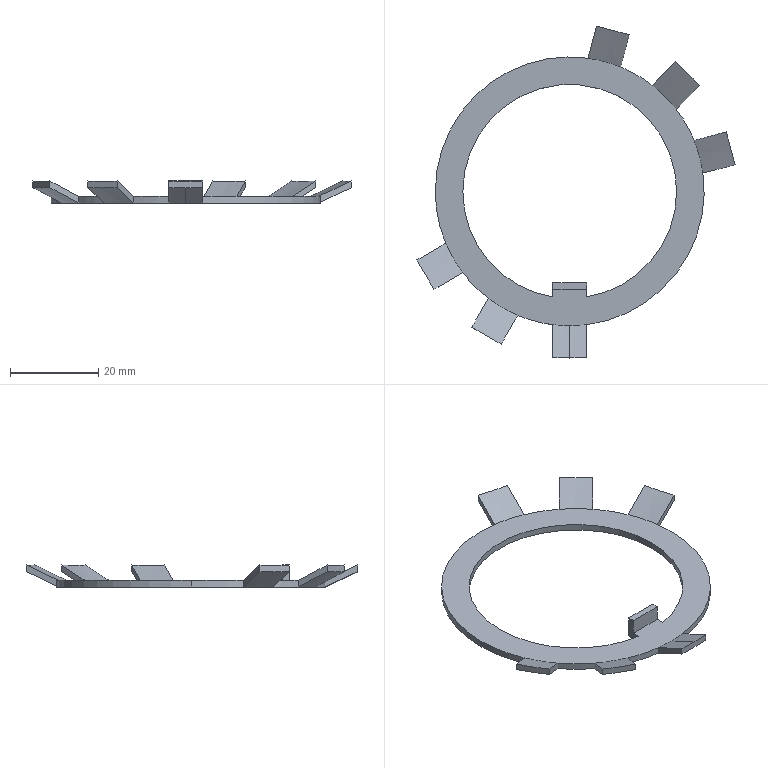Part | SolidWorks | features BaseBody 1 | 1 solid | 49 faces | box 72.177 x 75.317 x 5 mm | volume 2204 mm3 | plane 25 | cone 14 | cylinder 10 | commonest cylinder face diameters 61 x7 48.5 x3
STEP:
#1=CARTESIAN_POINT('',(0.,-30.5,0.));
#2=VERTEX_POINT('',#1);
#3=CARTESIAN_POINT('',(-3.85,-30.256,0.));
#4=VERTEX_POINT('',#3);
#5=CARTESIAN_POINT('',(0.,0.,0.));
#6=DIRECTION('',(0.,0.,-1.));
#7=DIRECTION('',(0.,1.,0.));
#8=AXIS2_PLACEMENT_3D('',#5,#6,#7);
#9=CIRCLE('',#8,30.5);
#10=EDGE_CURVE('',#2,#4,#9,.T.);
#11=ORIENTED_EDGE('',*,*,#10,.F.);
#12=CARTESIAN_POINT('',(0.,-37.804,3.406));
#13=VERTEX_POINT('',#12);
#14=CARTESIAN_POINT('',(0.,-30.5,0.));
#15=DIRECTION('',(0.,-0.9063,0.4226));
#16=VECTOR('',#15,1000.);
#17=LINE('',#14,#16);
#18=EDGE_CURVE('',#2,#13,#17,.T.);
#19=ORIENTED_EDGE('',*,*,#18,.T.);
#20=CARTESIAN_POINT('',(-3.85,-37.804,3.497));
#21=VERTEX_POINT('',#20);
#22=CARTESIAN_POINT('',(0.,-37.804,3.406));
#23=CARTESIAN_POINT('',(-1.282,-37.804,3.406));
#24=CARTESIAN_POINT('',(-2.567,-37.804,3.437));
#25=CARTESIAN_POINT('',(-3.85,-37.804,3.497));
#26=B_SPLINE_CURVE_WITH_KNOTS('',3,(#22,#23,#24,#25),.UNSPECIFIED.,.F.,.F.,(4,4),(0.01413,0.01797),.UNSPECIFIED.);
#27=EDGE_CURVE('',#13,#21,#26,.T.);
#28=ORIENTED_EDGE('',*,*,#27,.T.);
#29=CARTESIAN_POINT('',(-3.85,-37.804,3.497));
#30=CARTESIAN_POINT('',(-3.85,-35.289,2.33));
#31=CARTESIAN_POINT('',(-3.85,-32.773,1.164));
#32=CARTESIAN_POINT('',(-3.85,-30.256,0.));
#33=B_SPLINE_CURVE_WITH_KNOTS('',3,(#29,#30,#31,#32),.UNSPECIFIED.,.F.,.F.,(4,4),(0.01538,0.0237),.UNSPECIFIED.);
#34=EDGE_CURVE('',#21,#4,#33,.T.);
#35=ORIENTED_EDGE('',*,*,#34,.T.);
#36=EDGE_LOOP('',(#11,#19,#28,#35));
#37=FACE_OUTER_BOUND('',#36,.T.);
#38=CARTESIAN_POINT('',(0.,0.,0.));
#39=DIRECTION('',(0.,0.,1.));
#40=DIRECTION('',(0.,-1.,0.));
#41=AXIS2_PLACEMENT_3D('',#38,#39,#40);
#42=CONICAL_SURFACE('',#41,30.5,1.134);
#43=ADVANCED_FACE('',(#37),#42,.T.);
#44=CARTESIAN_POINT('',(-28.127,-11.794,1.5));
#45=VERTEX_POINT('',#44);
#46=CARTESIAN_POINT('',(-30.5,0.,1.5));
#47=VERTEX_POINT('',#46);
#48=CARTESIAN_POINT('',(0.,0.,1.5));
#49=DIRECTION('',(0.,0.,-1.));
#50=DIRECTION('',(0.,1.,0.));
#51=AXIS2_PLACEMENT_3D('',#48,#49,#50);
#52=CIRCLE('',#51,30.5);
#53=EDGE_CURVE('',#45,#47,#52,.T.);
#54=ORIENTED_EDGE('',*,*,#53,.T.);
#55=CARTESIAN_POINT('',(-30.5,0.,0.));
#56=VERTEX_POINT('',#55);
#57=CARTESIAN_POINT('',(-30.5,0.,4.998));
#58=DIRECTION('',(0.,0.,-1.));
#59=VECTOR('',#58,1000.);
#60=LINE('',#57,#59);
#61=EDGE_CURVE('',#47,#56,#60,.T.);
#62=ORIENTED_EDGE('',*,*,#61,.T.);
#63=CARTESIAN_POINT('',(-28.127,-11.794,0.));
#64=VERTEX_POINT('',#63);
#65=CARTESIAN_POINT('',(0.,0.,0.));
#66=DIRECTION('',(0.,0.,1.));
#67=DIRECTION('',(1.,0.,0.));
#68=AXIS2_PLACEMENT_3D('',#65,#66,#67);
#69=CIRCLE('',#68,30.5);
#70=EDGE_CURVE('',#56,#64,#69,.T.);
#71=ORIENTED_EDGE('',*,*,#70,.T.);
#72=CARTESIAN_POINT('',(-28.127,-11.794,4.998));
#73=DIRECTION('',(0.,0.,-1.));
#74=VECTOR('',#73,1000.);
#75=LINE('',#72,#74);
#76=EDGE_CURVE('',#45,#64,#75,.T.);
#77=ORIENTED_EDGE('',*,*,#76,.F.);
#78=EDGE_LOOP('',(#54,#62,#71,#77));
#79=FACE_OUTER_BOUND('',#78,.T.);
#80=CARTESIAN_POINT('',(0.,0.,4.998));
#81=DIRECTION('',(0.,0.,-1.));
#82=DIRECTION('',(-1.,0.,0.));
#83=AXIS2_PLACEMENT_3D('',#80,#81,#82);
#84=CYLINDRICAL_SURFACE('',#83,30.5);
#85=ADVANCED_FACE('',(#79),#84,.T.);
#86=CARTESIAN_POINT('',(3.85,-23.942,1.5));
#87=VERTEX_POINT('',#86);
#88=CARTESIAN_POINT('',(24.25,0.,1.5));
#89=VERTEX_POINT('',#88);
#90=CARTESIAN_POINT('',(0.,0.,1.5));
#91=DIRECTION('',(0.,0.,1.));
#92=DIRECTION('',(0.,-1.,0.));
#93=AXIS2_PLACEMENT_3D('',#90,#91,#92);
#94=CIRCLE('',#93,24.25);
#95=EDGE_CURVE('',#87,#89,#94,.T.);
#96=ORIENTED_EDGE('',*,*,#95,.T.);
#97=CARTESIAN_POINT('',(24.25,0.,0.));
#98=VERTEX_POINT('',#97);
#99=CARTESIAN_POINT('',(24.25,0.,4.998));
#100=DIRECTION('',(0.,0.,-1.));
#101=VECTOR('',#100,1000.);
#102=LINE('',#99,#101);
#103=EDGE_CURVE('',#89,#98,#102,.T.);
#104=ORIENTED_EDGE('',*,*,#103,.T.);
#105=CARTESIAN_POINT('',(3.85,-23.942,0.));
#106=VERTEX_POINT('',#105);
#107=CARTESIAN_POINT('',(0.,0.,0.));
#108=DIRECTION('',(0.,0.,1.));
#109=DIRECTION('',(1.,0.,0.));
#110=AXIS2_PLACEMENT_3D('',#107,#108,#109);
#111=CIRCLE('',#110,24.25);
#112=EDGE_CURVE('',#106,#98,#111,.T.);
#113=ORIENTED_EDGE('',*,*,#112,.F.);
#114=CARTESIAN_POINT('',(3.85,-23.942,4.998));
#115=DIRECTION('',(0.,0.,-1.));
#116=VECTOR('',#115,1000.);
#117=LINE('',#114,#116);
#118=EDGE_CURVE('',#87,#106,#117,.T.);
#119=ORIENTED_EDGE('',*,*,#118,.F.);
#120=EDGE_LOOP('',(#96,#104,#113,#119));
#121=FACE_OUTER_BOUND('',#120,.T.);
#122=CARTESIAN_POINT('',(0.,0.,4.998));
#123=DIRECTION('',(0.,0.,-1.));
#124=DIRECTION('',(-1.,0.,0.));
#125=AXIS2_PLACEMENT_3D('',#122,#123,#124);
#126=CYLINDRICAL_SURFACE('',#125,24.25);
#127=ADVANCED_FACE('',(#121),#126,.F.);
#128=ORIENTED_EDGE('',*,*,#103,.F.);
#129=CARTESIAN_POINT('',(-24.25,0.,1.5));
#130=VERTEX_POINT('',#129);
#131=CARTESIAN_POINT('',(0.,0.,1.5));
#132=DIRECTION('',(0.,0.,1.));
#133=DIRECTION('',(0.,-1.,0.));
#134=AXIS2_PLACEMENT_3D('',#131,#132,#133);
#135=CIRCLE('',#134,24.25);
#136=EDGE_CURVE('',#89,#130,#135,.T.);
#137=ORIENTED_EDGE('',*,*,#136,.T.);
#138=CARTESIAN_POINT('',(-24.25,0.,0.));
#139=VERTEX_POINT('',#138);
#140=CARTESIAN_POINT('',(-24.25,0.,4.998));
#141=DIRECTION('',(0.,0.,-1.));
#142=VECTOR('',#141,1000.);
#143=LINE('',#140,#142);
#144=EDGE_CURVE('',#130,#139,#143,.T.);
#145=ORIENTED_EDGE('',*,*,#144,.T.);
#146=CARTESIAN_POINT('',(0.,0.,0.));
#147=DIRECTION('',(0.,0.,1.));
#148=DIRECTION('',(1.,0.,0.));
#149=AXIS2_PLACEMENT_3D('',#146,#147,#148);
#150=CIRCLE('',#149,24.25);
#151=EDGE_CURVE('',#98,#139,#150,.T.);
#152=ORIENTED_EDGE('',*,*,#151,.F.);
#153=EDGE_LOOP('',(#128,#137,#145,#152));
#154=FACE_OUTER_BOUND('',#153,.T.);
#155=CARTESIAN_POINT('',(0.,0.,4.998));
#156=DIRECTION('',(0.,0.,-1.));
#157=DIRECTION('',(-1.,0.,0.));
#158=AXIS2_PLACEMENT_3D('',#155,#156,#157);
#159=CYLINDRICAL_SURFACE('',#158,24.25);
#160=ADVANCED_FACE('',(#154),#159,.F.);
#161=CARTESIAN_POINT('',(3.85,-30.256,1.5));
#162=VERTEX_POINT('',#161);
#163=CARTESIAN_POINT('',(0.,-30.5,1.5));
#164=VERTEX_POINT('',#163);
#165=CARTESIAN_POINT('',(0.,0.,1.5));
#166=DIRECTION('',(0.,0.,-1.));
#167=DIRECTION('',(0.,1.,0.));
#168=AXIS2_PLACEMENT_3D('',#165,#166,#167);
#169=CIRCLE('',#168,30.5);
#170=EDGE_CURVE('',#162,#164,#169,.T.);
#171=ORIENTED_EDGE('',*,*,#170,.T.);
#172=CARTESIAN_POINT('',(0.,-37.804,4.906));
#173=VERTEX_POINT('',#172);
#174=CARTESIAN_POINT('',(0.,-38.,4.997));
#175=DIRECTION('',(0.,-0.9063,0.4226));
#176=VECTOR('',#175,1000.);
#177=LINE('',#174,#176);
#178=EDGE_CURVE('',#164,#173,#177,.T.);
#179=ORIENTED_EDGE('',*,*,#178,.T.);
#180=CARTESIAN_POINT('',(3.85,-37.804,4.997));
#181=VERTEX_POINT('',#180);
#182=CARTESIAN_POINT('',(0.,-37.804,4.906));
#183=CARTESIAN_POINT('',(1.285,-37.804,4.906));
#184=CARTESIAN_POINT('',(2.569,-37.804,4.937));
#185=CARTESIAN_POINT('',(3.85,-37.804,4.997));
#186=B_SPLINE_CURVE_WITH_KNOTS('',3,(#182,#183,#184,#185),.UNSPECIFIED.,.F.,.F.,(4,4),(0.01982,0.02367),.UNSPECIFIED.);
#187=EDGE_CURVE('',#173,#181,#186,.T.);
#188=ORIENTED_EDGE('',*,*,#187,.T.);
#189=CARTESIAN_POINT('',(3.85,-37.804,4.997));
#190=CARTESIAN_POINT('',(3.85,-35.289,3.83));
#191=CARTESIAN_POINT('',(3.85,-32.773,2.664));
#192=CARTESIAN_POINT('',(3.85,-30.256,1.5));
#193=B_SPLINE_CURVE_WITH_KNOTS('',3,(#189,#190,#191,#192),.UNSPECIFIED.,.F.,.F.,(4,4),(0.01538,0.0237),.UNSPECIFIED.);
#194=EDGE_CURVE('',#181,#162,#193,.T.);
#195=ORIENTED_EDGE('',*,*,#194,.T.);
#196=EDGE_LOOP('',(#171,#179,#188,#195));
#197=FACE_OUTER_BOUND('',#196,.T.);
#198=CARTESIAN_POINT('',(0.,0.,4.997));
#199=DIRECTION('',(0.,0.,1.));
#200=DIRECTION('',(0.,-1.,0.));
#201=AXIS2_PLACEMENT_3D('',#198,#199,#200);
#202=CONICAL_SURFACE('',#201,38.,1.134);
#203=ADVANCED_FACE('',(#197),#202,.F.);
#204=CARTESIAN_POINT('',(4.112,30.222,1.5));
#205=VERTEX_POINT('',#204);
#206=CARTESIAN_POINT('',(11.55,28.229,1.5));
#207=VERTEX_POINT('',#206);
#208=CARTESIAN_POINT('',(0.,0.,1.5));
#209=DIRECTION('',(0.,0.,-1.));
#210=DIRECTION('',(0.,1.,0.));
#211=AXIS2_PLACEMENT_3D('',#208,#209,#210);
#212=CIRCLE('',#211,30.5);
#213=EDGE_CURVE('',#205,#207,#212,.T.);
#214=ORIENTED_EDGE('',*,*,#213,.F.);
#215=CARTESIAN_POINT('',(0.,0.,1.5));
#216=DIRECTION('',(0.,0.,-1.));
#217=DIRECTION('',(0.,1.,0.));
#218=AXIS2_PLACEMENT_3D('',#215,#216,#217);
#219=CIRCLE('',#218,30.5);
#220=EDGE_CURVE('',#47,#205,#219,.T.);
#221=ORIENTED_EDGE('',*,*,#220,.F.);
#222=ORIENTED_EDGE('',*,*,#53,.F.);
#223=CARTESIAN_POINT('',(-24.277,-18.462,1.5));
#224=VERTEX_POINT('',#223);
#225=CARTESIAN_POINT('',(0.,0.,1.5));
#226=DIRECTION('',(0.,0.,-1.));
#227=DIRECTION('',(0.,1.,0.));
#228=AXIS2_PLACEMENT_3D('',#225,#226,#227);
#229=CIRCLE('',#228,30.5);
#230=EDGE_CURVE('',#224,#45,#229,.T.);
#231=ORIENTED_EDGE('',*,*,#230,.F.);
#232=CARTESIAN_POINT('',(-18.462,-24.277,1.5));
#233=VERTEX_POINT('',#232);
#234=CARTESIAN_POINT('',(0.,0.,1.5));
#235=DIRECTION('',(0.,0.,-1.));
#236=DIRECTION('',(0.,1.,0.));
#237=AXIS2_PLACEMENT_3D('',#234,#235,#236);
#238=CIRCLE('',#237,30.5);
#239=EDGE_CURVE('',#233,#224,#238,.T.);
#240=ORIENTED_EDGE('',*,*,#239,.F.);
#241=CARTESIAN_POINT('',(-11.794,-28.127,1.5));
#242=VERTEX_POINT('',#241);
#243=CARTESIAN_POINT('',(0.,0.,1.5));
#244=DIRECTION('',(0.,0.,-1.));
#245=DIRECTION('',(0.,1.,0.));
#246=AXIS2_PLACEMENT_3D('',#243,#244,#245);
#247=CIRCLE('',#246,30.5);
#248=EDGE_CURVE('',#242,#233,#247,.T.);
#249=ORIENTED_EDGE('',*,*,#248,.F.);
#250=CARTESIAN_POINT('',(-3.85,-30.256,1.5));
#251=VERTEX_POINT('',#250);
#252=CARTESIAN_POINT('',(0.,0.,1.5));
#253=DIRECTION('',(0.,0.,-1.));
#254=DIRECTION('',(0.,1.,0.));
#255=AXIS2_PLACEMENT_3D('',#252,#253,#254);
#256=CIRCLE('',#255,30.5);
#257=EDGE_CURVE('',#251,#242,#256,.T.);
#258=ORIENTED_EDGE('',*,*,#257,.F.);
#259=CARTESIAN_POINT('',(0.,0.,1.5));
#260=DIRECTION('',(0.,0.,-1.));
#261=DIRECTION('',(0.,1.,0.));
#262=AXIS2_PLACEMENT_3D('',#259,#260,#261);
#263=CIRCLE('',#262,30.5);
#264=EDGE_CURVE('',#164,#251,#263,.T.);
#265=ORIENTED_EDGE('',*,*,#264,.F.);
#266=ORIENTED_EDGE('',*,*,#170,.F.);
#267=CARTESIAN_POINT('',(30.222,4.112,1.5));
#268=VERTEX_POINT('',#267);
#269=CARTESIAN_POINT('',(0.,0.,1.5));
#270=DIRECTION('',(0.,0.,-1.));
#271=DIRECTION('',(0.,1.,0.));
#272=AXIS2_PLACEMENT_3D('',#269,#270,#271);
#273=CIRCLE('',#272,30.5);
#274=EDGE_CURVE('',#268,#162,#273,.T.);
#275=ORIENTED_EDGE('',*,*,#274,.F.);
#276=CARTESIAN_POINT('',(28.229,11.55,1.5));
#277=VERTEX_POINT('',#276);
#278=CARTESIAN_POINT('',(0.,0.,1.5));
#279=DIRECTION('',(0.,0.,-1.));
#280=DIRECTION('',(0.,1.,0.));
#281=AXIS2_PLACEMENT_3D('',#278,#279,#280);
#282=CIRCLE('',#281,30.5);
#283=EDGE_CURVE('',#277,#268,#282,.T.);
#284=ORIENTED_EDGE('',*,*,#283,.F.);
#285=CARTESIAN_POINT('',(24.117,18.672,1.5));
#286=VERTEX_POINT('',#285);
#287=CARTESIAN_POINT('',(0.,0.,1.5));
#288=DIRECTION('',(0.,0.,-1.));
#289=DIRECTION('',(0.,1.,0.));
#290=AXIS2_PLACEMENT_3D('',#287,#288,#289);
#291=CIRCLE('',#290,30.5);
#292=EDGE_CURVE('',#286,#277,#291,.T.);
#293=ORIENTED_EDGE('',*,*,#292,.F.);
#294=CARTESIAN_POINT('',(18.672,24.117,1.5));
#295=VERTEX_POINT('',#294);
#296=CARTESIAN_POINT('',(0.,0.,1.5));
#297=DIRECTION('',(0.,0.,-1.));
#298=DIRECTION('',(0.,1.,0.));
#299=AXIS2_PLACEMENT_3D('',#296,#297,#298);
#300=CIRCLE('',#299,30.5);
#301=EDGE_CURVE('',#295,#286,#300,.T.);
#302=ORIENTED_EDGE('',*,*,#301,.F.);
#303=CARTESIAN_POINT('',(0.,0.,1.5));
#304=DIRECTION('',(0.,0.,-1.));
#305=DIRECTION('',(0.,1.,0.));
#306=AXIS2_PLACEMENT_3D('',#303,#304,#305);
#307=CIRCLE('',#306,30.5);
#308=EDGE_CURVE('',#207,#295,#307,.T.);
#309=ORIENTED_EDGE('',*,*,#308,.F.);
#310=EDGE_LOOP('',(#214,#221,#222,#231,#240,#249,#258,#265,#266,#275,#284,#293,#302,#309));
#311=FACE_OUTER_BOUND('',#310,.T.);
#312=CARTESIAN_POINT('',(3.85,-22.25,1.5));
#313=VERTEX_POINT('',#312);
#314=CARTESIAN_POINT('',(3.85,-23.942,1.5));
#315=DIRECTION('',(0.,-1.,0.));
#316=VECTOR('',#315,1000.);
#317=LINE('',#314,#316);
#318=EDGE_CURVE('',#313,#87,#317,.T.);
#319=ORIENTED_EDGE('',*,*,#318,.F.);
#320=CARTESIAN_POINT('',(-3.85,-22.25,1.5));
#321=VERTEX_POINT('',#320);
#322=CARTESIAN_POINT('',(0.,-22.25,1.5));
#323=DIRECTION('',(-1.,0.,0.));
#324=VECTOR('',#323,1000.);
#325=LINE('',#322,#324);
#326=EDGE_CURVE('',#313,#321,#325,.T.);
#327=ORIENTED_EDGE('',*,*,#326,.T.);
#328=CARTESIAN_POINT('',(-3.85,-23.942,1.5));
#329=VERTEX_POINT('',#328);
#330=CARTESIAN_POINT('',(-3.85,-23.942,1.5));
#331=DIRECTION('',(0.,1.,0.));
#332=VECTOR('',#331,1000.);
#333=LINE('',#330,#332);
#334=EDGE_CURVE('',#329,#321,#333,.T.);
#335=ORIENTED_EDGE('',*,*,#334,.F.);
#336=CARTESIAN_POINT('',(0.,0.,1.5));
#337=DIRECTION('',(0.,0.,1.));
#338=DIRECTION('',(0.,-1.,0.));
#339=AXIS2_PLACEMENT_3D('',#336,#337,#338);
#340=CIRCLE('',#339,24.25);
#341=EDGE_CURVE('',#130,#329,#340,.T.);
#342=ORIENTED_EDGE('',*,*,#341,.F.);
#343=ORIENTED_EDGE('',*,*,#136,.F.);
#344=ORIENTED_EDGE('',*,*,#95,.F.);
#345=EDGE_LOOP('',(#319,#327,#335,#342,#343,#344));
#346=FACE_BOUND('',#345,.T.);
#347=CARTESIAN_POINT('',(0.,30.5,1.5));
#348=DIRECTION('',(0.,0.,1.));
#349=DIRECTION('',(0.,-1.,0.));
#350=AXIS2_PLACEMENT_3D('',#347,#348,#349);
#351=PLANE('',#350);
#352=ADVANCED_FACE('',(#311,#346),#351,.T.);
#353=ORIENTED_EDGE('',*,*,#178,.F.);
#354=ORIENTED_EDGE('',*,*,#264,.T.);
#355=CARTESIAN_POINT('',(-3.85,-37.804,4.997));
#356=VERTEX_POINT('',#355);
#357=CARTESIAN_POINT('',(-3.85,-30.256,1.5));
#358=CARTESIAN_POINT('',(-3.85,-32.773,2.664));
#359=CARTESIAN_POINT('',(-3.85,-35.289,3.83));
#360=CARTESIAN_POINT('',(-3.85,-37.804,4.997));
#361=B_SPLINE_CURVE_WITH_KNOTS('',3,(#357,#358,#359,#360),.UNSPECIFIED.,.F.,.F.,(4,4),(0.009504,0.01782),.UNSPECIFIED.);
#362=EDGE_CURVE('',#251,#356,#361,.T.);
#363=ORIENTED_EDGE('',*,*,#362,.T.);
#364=CARTESIAN_POINT('',(-3.85,-37.804,4.997));
#365=CARTESIAN_POINT('',(-2.567,-37.804,4.937));
#366=CARTESIAN_POINT('',(-1.282,-37.804,4.906));
#367=CARTESIAN_POINT('',(0.,-37.804,4.906));
#368=B_SPLINE_CURVE_WITH_KNOTS('',3,(#364,#365,#366,#367),.UNSPECIFIED.,.F.,.F.,(4,4),(0.01598,0.01982),.UNSPECIFIED.);
#369=EDGE_CURVE('',#356,#173,#368,.T.);
#370=ORIENTED_EDGE('',*,*,#369,.T.);
#371=EDGE_LOOP('',(#353,#354,#363,#370));
#372=FACE_OUTER_BOUND('',#371,.T.);
#373=CARTESIAN_POINT('',(0.,0.,4.997));
#374=DIRECTION('',(0.,0.,1.));
#375=DIRECTION('',(0.,-1.,0.));
#376=AXIS2_PLACEMENT_3D('',#373,#374,#375);
#377=CONICAL_SURFACE('',#376,38.,1.134);
#378=ADVANCED_FACE('',(#372),#377,.F.);
#379=CARTESIAN_POINT('',(-22.236,-30.815,4.997));
#380=VERTEX_POINT('',#379);
#381=CARTESIAN_POINT('',(-18.462,-24.277,1.5));
#382=CARTESIAN_POINT('',(-19.721,-26.457,2.664));
#383=CARTESIAN_POINT('',(-20.979,-28.636,3.83));
#384=CARTESIAN_POINT('',(-22.236,-30.815,4.997));
#385=B_SPLINE_CURVE_WITH_KNOTS('',3,(#381,#382,#383,#384),.UNSPECIFIED.,.F.,.F.,(4,4),(0.000000255,0.00832),.UNSPECIFIED.);
#386=EDGE_CURVE('',#233,#380,#385,.T.);
#387=ORIENTED_EDGE('',*,*,#386,.T.);
#388=CARTESIAN_POINT('',(-15.568,-34.665,4.997));
#389=VERTEX_POINT('',#388);
#390=CARTESIAN_POINT('',(-22.236,-30.815,4.997));
#391=CARTESIAN_POINT('',(-20.014,-32.098,4.876));
#392=CARTESIAN_POINT('',(-17.791,-33.381,4.876));
#393=CARTESIAN_POINT('',(-15.568,-34.665,4.997));
#394=B_SPLINE_CURVE_WITH_KNOTS('',3,(#390,#391,#392,#393),.UNSPECIFIED.,.F.,.F.,(4,4),(0.000000231,0.0077),.UNSPECIFIED.);
#395=EDGE_CURVE('',#380,#389,#394,.T.);
#396=ORIENTED_EDGE('',*,*,#395,.T.);
#397=CARTESIAN_POINT('',(-15.568,-34.665,4.997));
#398=CARTESIAN_POINT('',(-14.31,-32.486,3.83));
#399=CARTESIAN_POINT('',(-13.052,-30.307,2.664));
#400=CARTESIAN_POINT('',(-11.794,-28.127,1.5));
#401=B_SPLINE_CURVE_WITH_KNOTS('',3,(#397,#398,#399,#400),.UNSPECIFIED.,.F.,.F.,(4,4),(0.000000255,0.00832),.UNSPECIFIED.);
#402=EDGE_CURVE('',#389,#242,#401,.T.);
#403=ORIENTED_EDGE('',*,*,#402,.T.);
#404=ORIENTED_EDGE('',*,*,#248,.T.);
#405=EDGE_LOOP('',(#387,#396,#403,#404));
#406=FACE_OUTER_BOUND('',#405,.T.);
#407=CARTESIAN_POINT('',(0.,0.,4.997));
#408=DIRECTION('',(0.,0.,1.));
#409=DIRECTION('',(0.,-1.,0.));
#410=AXIS2_PLACEMENT_3D('',#407,#408,#409);
#411=CONICAL_SURFACE('',#410,38.,1.134);
#412=ADVANCED_FACE('',(#406),#411,.F.);
#413=CARTESIAN_POINT('',(-34.665,-15.568,4.997));
#414=VERTEX_POINT('',#413);
#415=CARTESIAN_POINT('',(-28.127,-11.794,1.5));
#416=CARTESIAN_POINT('',(-30.307,-13.052,2.664));
#417=CARTESIAN_POINT('',(-32.486,-14.31,3.83));
#418=CARTESIAN_POINT('',(-34.665,-15.568,4.997));
#419=B_SPLINE_CURVE_WITH_KNOTS('',3,(#415,#416,#417,#418),.UNSPECIFIED.,.F.,.F.,(4,4),(0.000000255,0.00832),.UNSPECIFIED.);
#420=EDGE_CURVE('',#45,#414,#419,.T.);
#421=ORIENTED_EDGE('',*,*,#420,.T.);
#422=CARTESIAN_POINT('',(-30.815,-22.236,4.997));
#423=VERTEX_POINT('',#422);
#424=CARTESIAN_POINT('',(-34.665,-15.568,4.997));
#425=CARTESIAN_POINT('',(-33.381,-17.791,4.876));
#426=CARTESIAN_POINT('',(-32.098,-20.014,4.876));
#427=CARTESIAN_POINT('',(-30.815,-22.236,4.997));
#428=B_SPLINE_CURVE_WITH_KNOTS('',3,(#424,#425,#426,#427),.UNSPECIFIED.,.F.,.F.,(4,4),(0.000000231,0.0077),.UNSPECIFIED.);
#429=EDGE_CURVE('',#414,#423,#428,.T.);
#430=ORIENTED_EDGE('',*,*,#429,.T.);
#431=CARTESIAN_POINT('',(-30.815,-22.236,4.997));
#432=CARTESIAN_POINT('',(-28.636,-20.979,3.83));
#433=CARTESIAN_POINT('',(-26.457,-19.721,2.664));
#434=CARTESIAN_POINT('',(-24.277,-18.462,1.5));
#435=B_SPLINE_CURVE_WITH_KNOTS('',3,(#431,#432,#433,#434),.UNSPECIFIED.,.F.,.F.,(4,4),(0.000000255,0.00832),.UNSPECIFIED.);
#436=EDGE_CURVE('',#423,#224,#435,.T.);
#437=ORIENTED_EDGE('',*,*,#436,.T.);
#438=ORIENTED_EDGE('',*,*,#230,.T.);
#439=EDGE_LOOP('',(#421,#430,#437,#438));
#440=FACE_OUTER_BOUND('',#439,.T.);
#441=CARTESIAN_POINT('',(0.,0.,4.997));
#442=DIRECTION('',(0.,0.,1.));
#443=DIRECTION('',(0.,-1.,0.));
#444=AXIS2_PLACEMENT_3D('',#441,#442,#443);
#445=CONICAL_SURFACE('',#444,38.,1.134);
#446=ADVANCED_FACE('',(#440),#445,.F.);
#447=CARTESIAN_POINT('',(13.503,35.52,4.997));
#448=VERTEX_POINT('',#447);
#449=CARTESIAN_POINT('',(11.55,28.229,1.5));
#450=CARTESIAN_POINT('',(12.201,30.66,2.664));
#451=CARTESIAN_POINT('',(12.852,33.09,3.83));
#452=CARTESIAN_POINT('',(13.503,35.52,4.997));
#453=B_SPLINE_CURVE_WITH_KNOTS('',3,(#449,#450,#451,#452),.UNSPECIFIED.,.F.,.F.,(4,4),(0.000000228,0.008319),.UNSPECIFIED.);
#454=EDGE_CURVE('',#207,#448,#453,.T.);
#455=ORIENTED_EDGE('',*,*,#454,.T.);
#456=CARTESIAN_POINT('',(6.066,37.513,4.997));
#457=VERTEX_POINT('',#456);
#458=CARTESIAN_POINT('',(13.503,35.52,4.997));
#459=CARTESIAN_POINT('',(11.024,36.184,4.876));
#460=CARTESIAN_POINT('',(8.545,36.848,4.876));
#461=CARTESIAN_POINT('',(6.066,37.513,4.997));
#462=B_SPLINE_CURVE_WITH_KNOTS('',3,(#458,#459,#460,#461),.UNSPECIFIED.,.F.,.F.,(4,4),(0.000000207,0.0077),.UNSPECIFIED.);
#463=EDGE_CURVE('',#448,#457,#462,.T.);
#464=ORIENTED_EDGE('',*,*,#463,.T.);
#465=CARTESIAN_POINT('',(6.066,37.513,4.997));
#466=CARTESIAN_POINT('',(5.415,35.083,3.83));
#467=CARTESIAN_POINT('',(4.763,32.653,2.664));
#468=CARTESIAN_POINT('',(4.112,30.222,1.5));
#469=B_SPLINE_CURVE_WITH_KNOTS('',3,(#465,#466,#467,#468),.UNSPECIFIED.,.F.,.F.,(4,4),(0.000000228,0.008319),.UNSPECIFIED.);
#470=EDGE_CURVE('',#457,#205,#469,.T.);
#471=ORIENTED_EDGE('',*,*,#470,.T.);
#472=ORIENTED_EDGE('',*,*,#213,.T.);
#473=EDGE_LOOP('',(#455,#464,#471,#472));
#474=FACE_OUTER_BOUND('',#473,.T.);
#475=CARTESIAN_POINT('',(0.,0.,4.997));
#476=DIRECTION('',(0.,0.,1.));
#477=DIRECTION('',(0.,-1.,0.));
#478=AXIS2_PLACEMENT_3D('',#475,#476,#477);
#479=CONICAL_SURFACE('',#478,38.,1.134);
#480=ADVANCED_FACE('',(#474),#479,.F.);
#481=CARTESIAN_POINT('',(29.454,24.009,4.997));
#482=VERTEX_POINT('',#481);
#483=CARTESIAN_POINT('',(24.117,18.672,1.5));
#484=CARTESIAN_POINT('',(25.896,20.452,2.664));
#485=CARTESIAN_POINT('',(27.675,22.231,3.83));
#486=CARTESIAN_POINT('',(29.454,24.009,4.997));
#487=B_SPLINE_CURVE_WITH_KNOTS('',3,(#483,#484,#485,#486),.UNSPECIFIED.,.F.,.F.,(4,4),(0.000000312,0.00832),.UNSPECIFIED.);
#488=EDGE_CURVE('',#286,#482,#487,.T.);
#489=ORIENTED_EDGE('',*,*,#488,.T.);
#490=CARTESIAN_POINT('',(24.009,29.454,4.997));
#491=VERTEX_POINT('',#490);
#492=CARTESIAN_POINT('',(29.454,24.009,4.997));
#493=CARTESIAN_POINT('',(27.639,25.824,4.876));
#494=CARTESIAN_POINT('',(25.824,27.639,4.876));
#495=CARTESIAN_POINT('',(24.009,29.454,4.997));
#496=B_SPLINE_CURVE_WITH_KNOTS('',3,(#492,#493,#494,#495),.UNSPECIFIED.,.F.,.F.,(4,4),(0.000000283,0.0077),.UNSPECIFIED.);
#497=EDGE_CURVE('',#482,#491,#496,.T.);
#498=ORIENTED_EDGE('',*,*,#497,.T.);
#499=CARTESIAN_POINT('',(24.009,29.454,4.997));
#500=CARTESIAN_POINT('',(22.231,27.675,3.83));
#501=CARTESIAN_POINT('',(20.452,25.896,2.664));
#502=CARTESIAN_POINT('',(18.672,24.117,1.5));
#503=B_SPLINE_CURVE_WITH_KNOTS('',3,(#499,#500,#501,#502),.UNSPECIFIED.,.F.,.F.,(4,4),(0.000000312,0.00832),.UNSPECIFIED.);
#504=EDGE_CURVE('',#491,#295,#503,.T.);
#505=ORIENTED_EDGE('',*,*,#504,.T.);
#506=ORIENTED_EDGE('',*,*,#301,.T.);
#507=EDGE_LOOP('',(#489,#498,#505,#506));
#508=FACE_OUTER_BOUND('',#507,.T.);
#509=CARTESIAN_POINT('',(0.,0.,4.997));
#510=DIRECTION('',(0.,0.,1.));
#511=DIRECTION('',(0.,-1.,0.));
#512=AXIS2_PLACEMENT_3D('',#509,#510,#511);
#513=CONICAL_SURFACE('',#512,38.,1.134);
#514=ADVANCED_FACE('',(#508),#513,.F.);
#515=CARTESIAN_POINT('',(37.513,6.066,4.997));
#516=VERTEX_POINT('',#515);
#517=CARTESIAN_POINT('',(30.222,4.112,1.5));
#518=CARTESIAN_POINT('',(32.653,4.763,2.664));
#519=CARTESIAN_POINT('',(35.083,5.415,3.83));
#520=CARTESIAN_POINT('',(37.513,6.066,4.997));
#521=B_SPLINE_CURVE_WITH_KNOTS('',3,(#517,#518,#519,#520),.UNSPECIFIED.,.F.,.F.,(4,4),(0.000000228,0.008319),.UNSPECIFIED.);
#522=EDGE_CURVE('',#268,#516,#521,.T.);
#523=ORIENTED_EDGE('',*,*,#522,.T.);
#524=CARTESIAN_POINT('',(35.52,13.503,4.997));
#525=VERTEX_POINT('',#524);
#526=CARTESIAN_POINT('',(37.513,6.066,4.997));
#527=CARTESIAN_POINT('',(36.848,8.545,4.876));
#528=CARTESIAN_POINT('',(36.184,11.024,4.876));
#529=CARTESIAN_POINT('',(35.52,13.503,4.997));
#530=B_SPLINE_CURVE_WITH_KNOTS('',3,(#526,#527,#528,#529),.UNSPECIFIED.,.F.,.F.,(4,4),(0.000000207,0.0077),.UNSPECIFIED.);
#531=EDGE_CURVE('',#516,#525,#530,.T.);
#532=ORIENTED_EDGE('',*,*,#531,.T.);
#533=CARTESIAN_POINT('',(35.52,13.503,4.997));
#534=CARTESIAN_POINT('',(33.09,12.852,3.83));
#535=CARTESIAN_POINT('',(30.66,12.201,2.664));
#536=CARTESIAN_POINT('',(28.229,11.55,1.5));
#537=B_SPLINE_CURVE_WITH_KNOTS('',3,(#533,#534,#535,#536),.UNSPECIFIED.,.F.,.F.,(4,4),(0.000000228,0.008319),.UNSPECIFIED.);
#538=EDGE_CURVE('',#525,#277,#537,.T.);
#539=ORIENTED_EDGE('',*,*,#538,.T.);
#540=ORIENTED_EDGE('',*,*,#283,.T.);
#541=EDGE_LOOP('',(#523,#532,#539,#540));
#542=FACE_OUTER_BOUND('',#541,.T.);
#543=CARTESIAN_POINT('',(0.,0.,4.997));
#544=DIRECTION('',(0.,0.,1.));
#545=DIRECTION('',(0.,-1.,0.));
#546=AXIS2_PLACEMENT_3D('',#543,#544,#545);
#547=CONICAL_SURFACE('',#546,38.,1.134);
#548=ADVANCED_FACE('',(#542),#547,.F.);
#549=CARTESIAN_POINT('',(3.85,-20.75,5.));
#550=VERTEX_POINT('',#549);
#551=CARTESIAN_POINT('',(3.85,-20.75,0.));
#552=VERTEX_POINT('',#551);
#553=CARTESIAN_POINT('',(3.85,-20.75,4.998));
#554=DIRECTION('',(0.,0.,-1.));
#555=VECTOR('',#554,1000.);
#556=LINE('',#553,#555);
#557=EDGE_CURVE('',#550,#552,#556,.T.);
#558=ORIENTED_EDGE('',*,*,#557,.F.);
#559=CARTESIAN_POINT('',(3.85,-22.25,5.));
#560=VERTEX_POINT('',#559);
#561=CARTESIAN_POINT('',(3.85,-20.75,5.));
#562=DIRECTION('',(0.,1.,0.));
#563=VECTOR('',#562,1000.);
#564=LINE('',#561,#563);
#565=EDGE_CURVE('',#560,#550,#564,.T.);
#566=ORIENTED_EDGE('',*,*,#565,.F.);
#567=CARTESIAN_POINT('',(3.85,-22.25,5.));
#568=DIRECTION('',(0.,0.,-1.));
#569=VECTOR('',#568,1000.);
#570=LINE('',#567,#569);
#571=EDGE_CURVE('',#560,#313,#570,.T.);
#572=ORIENTED_EDGE('',*,*,#571,.T.);
#573=ORIENTED_EDGE('',*,*,#318,.T.);
#574=ORIENTED_EDGE('',*,*,#118,.T.);
#575=CARTESIAN_POINT('',(3.85,-23.942,0.));
#576=DIRECTION('',(0.,-1.,0.));
#577=VECTOR('',#576,1000.);
#578=LINE('',#575,#577);
#579=EDGE_CURVE('',#552,#106,#578,.T.);
#580=ORIENTED_EDGE('',*,*,#579,.F.);
#581=EDGE_LOOP('',(#558,#566,#572,#573,#574,#580));
#582=FACE_OUTER_BOUND('',#581,.T.);
#583=CARTESIAN_POINT('',(3.85,-23.942,4.998));
#584=DIRECTION('',(1.,0.,0.));
#585=DIRECTION('',(0.,1.,0.));
#586=AXIS2_PLACEMENT_3D('',#583,#584,#585);
#587=PLANE('',#586);
#588=ADVANCED_FACE('',(#582),#587,.T.);
#589=CARTESIAN_POINT('',(-3.85,-20.75,5.));
#590=VERTEX_POINT('',#589);
#591=CARTESIAN_POINT('',(-3.85,-20.75,0.));
#592=VERTEX_POINT('',#591);
#593=CARTESIAN_POINT('',(-3.85,-20.75,4.998));
#594=DIRECTION('',(0.,0.,-1.));
#595=VECTOR('',#594,1000.);
#596=LINE('',#593,#595);
#597=EDGE_CURVE('',#590,#592,#596,.T.);
#598=ORIENTED_EDGE('',*,*,#597,.F.);
#599=CARTESIAN_POINT('',(-3.85,-20.75,5.));
#600=DIRECTION('',(-1.,0.,0.));
#601=VECTOR('',#600,1000.);
#602=LINE('',#599,#601);
#603=EDGE_CURVE('',#550,#590,#602,.T.);
#604=ORIENTED_EDGE('',*,*,#603,.F.);
#605=ORIENTED_EDGE('',*,*,#557,.T.);
#606=CARTESIAN_POINT('',(3.85,-20.75,0.));
#607=DIRECTION('',(1.,0.,0.));
#608=VECTOR('',#607,1000.);
#609=LINE('',#606,#608);
#610=EDGE_CURVE('',#592,#552,#609,.T.);
#611=ORIENTED_EDGE('',*,*,#610,.F.);
#612=EDGE_LOOP('',(#598,#604,#605,#611));
#613=FACE_OUTER_BOUND('',#612,.T.);
#614=CARTESIAN_POINT('',(3.85,-20.75,4.998));
#615=DIRECTION('',(0.,1.,0.));
#616=DIRECTION('',(0.,0.,1.));
#617=AXIS2_PLACEMENT_3D('',#614,#615,#616);
#618=PLANE('',#617);
#619=ADVANCED_FACE('',(#613),#618,.T.);
#620=ORIENTED_EDGE('',*,*,#597,.T.);
#621=CARTESIAN_POINT('',(-3.85,-23.942,0.));
#622=VERTEX_POINT('',#621);
#623=CARTESIAN_POINT('',(-3.85,-23.942,0.));
#624=DIRECTION('',(0.,1.,0.));
#625=VECTOR('',#624,1000.);
#626=LINE('',#623,#625);
#627=EDGE_CURVE('',#622,#592,#626,.T.);
#628=ORIENTED_EDGE('',*,*,#627,.F.);
#629=CARTESIAN_POINT('',(-3.85,-23.942,4.998));
#630=DIRECTION('',(0.,0.,-1.));
#631=VECTOR('',#630,1000.);
#632=LINE('',#629,#631);
#633=EDGE_CURVE('',#329,#622,#632,.T.);
#634=ORIENTED_EDGE('',*,*,#633,.F.);
#635=ORIENTED_EDGE('',*,*,#334,.T.);
#636=CARTESIAN_POINT('',(-3.85,-22.25,5.));
#637=VERTEX_POINT('',#636);
#638=CARTESIAN_POINT('',(-3.85,-22.25,5.));
#639=DIRECTION('',(0.,0.,-1.));
#640=VECTOR('',#639,1000.);
#641=LINE('',#638,#640);
#642=EDGE_CURVE('',#637,#321,#641,.T.);
#643=ORIENTED_EDGE('',*,*,#642,.F.);
#644=CARTESIAN_POINT('',(-3.85,-20.75,5.));
#645=DIRECTION('',(0.,-1.,0.));
#646=VECTOR('',#645,1000.);
#647=LINE('',#644,#646);
#648=EDGE_CURVE('',#590,#637,#647,.T.);
#649=ORIENTED_EDGE('',*,*,#648,.F.);
#650=EDGE_LOOP('',(#620,#628,#634,#635,#643,#649));
#651=FACE_OUTER_BOUND('',#650,.T.);
#652=CARTESIAN_POINT('',(-3.85,-23.942,4.998));
#653=DIRECTION('',(-1.,0.,0.));
#654=DIRECTION('',(0.,-1.,0.));
#655=AXIS2_PLACEMENT_3D('',#652,#653,#654);
#656=PLANE('',#655);
#657=ADVANCED_FACE('',(#651),#656,.T.);
#658=ORIENTED_EDGE('',*,*,#144,.F.);
#659=ORIENTED_EDGE('',*,*,#341,.T.);
#660=ORIENTED_EDGE('',*,*,#633,.T.);
#661=CARTESIAN_POINT('',(0.,0.,0.));
#662=DIRECTION('',(0.,0.,1.));
#663=DIRECTION('',(1.,0.,0.));
#664=AXIS2_PLACEMENT_3D('',#661,#662,#663);
#665=CIRCLE('',#664,24.25);
#666=EDGE_CURVE('',#139,#622,#665,.T.);
#667=ORIENTED_EDGE('',*,*,#666,.F.);
#668=EDGE_LOOP('',(#658,#659,#660,#667));
#669=FACE_OUTER_BOUND('',#668,.T.);
#670=CARTESIAN_POINT('',(0.,0.,4.998));
#671=DIRECTION('',(0.,0.,-1.));
#672=DIRECTION('',(-1.,0.,0.));
#673=AXIS2_PLACEMENT_3D('',#670,#671,#672);
#674=CYLINDRICAL_SURFACE('',#673,24.25);
#675=ADVANCED_FACE('',(#669),#674,.F.);
#676=CARTESIAN_POINT('',(3.85,-30.256,0.));
#677=VERTEX_POINT('',#676);
#678=CARTESIAN_POINT('',(3.85,-37.804,3.497));
#679=VERTEX_POINT('',#678);
#680=CARTESIAN_POINT('',(3.85,-30.256,0.));
#681=CARTESIAN_POINT('',(3.85,-32.773,1.164));
#682=CARTESIAN_POINT('',(3.85,-35.289,2.33));
#683=CARTESIAN_POINT('',(3.85,-37.804,3.497));
#684=B_SPLINE_CURVE_WITH_KNOTS('',3,(#680,#681,#682,#683),.UNSPECIFIED.,.F.,.F.,(4,4),(0.009504,0.01782),.UNSPECIFIED.);
#685=EDGE_CURVE('',#677,#679,#684,.T.);
#686=ORIENTED_EDGE('',*,*,#685,.F.);
#687=CARTESIAN_POINT('',(3.85,-30.256,4.998));
#688=DIRECTION('',(0.,0.,-1.));
#689=VECTOR('',#688,1000.);
#690=LINE('',#687,#689);
#691=EDGE_CURVE('',#162,#677,#690,.T.);
#692=ORIENTED_EDGE('',*,*,#691,.F.);
#693=ORIENTED_EDGE('',*,*,#194,.F.);
#694=CARTESIAN_POINT('',(3.85,-37.804,4.998));
#695=DIRECTION('',(0.,0.,-1.));
#696=VECTOR('',#695,1000.);
#697=LINE('',#694,#696);
#698=EDGE_CURVE('',#181,#679,#697,.T.);
#699=ORIENTED_EDGE('',*,*,#698,.T.);
#700=EDGE_LOOP('',(#686,#692,#693,#699));
#701=FACE_OUTER_BOUND('',#700,.T.);
#702=CARTESIAN_POINT('',(3.85,-30.256,4.998));
#703=DIRECTION('',(-1.,0.,0.));
#704=DIRECTION('',(0.,-1.,0.));
#705=AXIS2_PLACEMENT_3D('',#702,#703,#704);
#706=PLANE('',#705);
#707=ADVANCED_FACE('',(#701),#706,.F.);
#708=ORIENTED_EDGE('',*,*,#274,.T.);
#709=ORIENTED_EDGE('',*,*,#691,.T.);
#710=CARTESIAN_POINT('',(30.222,4.112,0.));
#711=VERTEX_POINT('',#710);
#712=CARTESIAN_POINT('',(0.,0.,0.));
#713=DIRECTION('',(0.,0.,1.));
#714=DIRECTION('',(1.,0.,0.));
#715=AXIS2_PLACEMENT_3D('',#712,#713,#714);
#716=CIRCLE('',#715,30.5);
#717=EDGE_CURVE('',#677,#711,#716,.T.);
#718=ORIENTED_EDGE('',*,*,#717,.T.);
#719=CARTESIAN_POINT('',(30.222,4.112,4.998));
#720=DIRECTION('',(0.,0.,-1.));
#721=VECTOR('',#720,1000.);
#722=LINE('',#719,#721);
#723=EDGE_CURVE('',#268,#711,#722,.T.);
#724=ORIENTED_EDGE('',*,*,#723,.F.);
#725=EDGE_LOOP('',(#708,#709,#718,#724));
#726=FACE_OUTER_BOUND('',#725,.T.);
#727=CARTESIAN_POINT('',(0.,0.,4.998));
#728=DIRECTION('',(0.,0.,-1.));
#729=DIRECTION('',(-1.,0.,0.));
#730=AXIS2_PLACEMENT_3D('',#727,#728,#729);
#731=CYLINDRICAL_SURFACE('',#730,30.5);
#732=ADVANCED_FACE('',(#726),#731,.T.);
#733=CARTESIAN_POINT('',(37.513,6.066,3.497));
#734=VERTEX_POINT('',#733);
#735=CARTESIAN_POINT('',(37.513,6.066,3.497));
#736=CARTESIAN_POINT('',(35.083,5.415,2.33));
#737=CARTESIAN_POINT('',(32.653,4.763,1.164));
#738=CARTESIAN_POINT('',(30.222,4.112,0.));
#739=B_SPLINE_CURVE_WITH_KNOTS('',3,(#735,#736,#737,#738),.UNSPECIFIED.,.F.,.F.,(4,4),(0.000000228,0.008319),.UNSPECIFIED.);
#740=EDGE_CURVE('',#734,#711,#739,.T.);
#741=ORIENTED_EDGE('',*,*,#740,.F.);
#742=CARTESIAN_POINT('',(37.513,6.066,4.998));
#743=DIRECTION('',(0.,0.,-1.));
#744=VECTOR('',#743,1000.);
#745=LINE('',#742,#744);
#746=EDGE_CURVE('',#516,#734,#745,.T.);
#747=ORIENTED_EDGE('',*,*,#746,.F.);
#748=ORIENTED_EDGE('',*,*,#522,.F.);
#749=ORIENTED_EDGE('',*,*,#723,.T.);
#750=EDGE_LOOP('',(#741,#747,#748,#749));
#751=FACE_OUTER_BOUND('',#750,.T.);
#752=CARTESIAN_POINT('',(30.222,4.112,4.998));
#753=DIRECTION('',(-0.2588,0.9659,0.));
#754=DIRECTION('',(-0.9659,-0.2588,0.));
#755=AXIS2_PLACEMENT_3D('',#752,#753,#754);
#756=PLANE('',#755);
#757=ADVANCED_FACE('',(#751),#756,.F.);
#758=CARTESIAN_POINT('',(35.52,13.503,3.497));
#759=VERTEX_POINT('',#758);
#760=CARTESIAN_POINT('',(35.52,13.503,3.497));
#761=CARTESIAN_POINT('',(36.184,11.024,3.376));
#762=CARTESIAN_POINT('',(36.848,8.545,3.376));
#763=CARTESIAN_POINT('',(37.513,6.066,3.497));
#764=B_SPLINE_CURVE_WITH_KNOTS('',3,(#760,#761,#762,#763),.UNSPECIFIED.,.F.,.F.,(4,4),(0.000000207,0.0077),.UNSPECIFIED.);
#765=EDGE_CURVE('',#759,#734,#764,.T.);
#766=ORIENTED_EDGE('',*,*,#765,.F.);
#767=CARTESIAN_POINT('',(35.52,13.503,4.998));
#768=DIRECTION('',(0.,0.,-1.));
#769=VECTOR('',#768,1000.);
#770=LINE('',#767,#769);
#771=EDGE_CURVE('',#525,#759,#770,.T.);
#772=ORIENTED_EDGE('',*,*,#771,.F.);
#773=ORIENTED_EDGE('',*,*,#531,.F.);
#774=ORIENTED_EDGE('',*,*,#746,.T.);
#775=EDGE_LOOP('',(#766,#772,#773,#774));
#776=FACE_OUTER_BOUND('',#775,.T.);
#777=CARTESIAN_POINT('',(35.52,13.503,4.998));
#778=DIRECTION('',(-0.9659,-0.2588,0.));
#779=DIRECTION('',(0.2588,-0.9659,0.));
#780=AXIS2_PLACEMENT_3D('',#777,#778,#779);
#781=PLANE('',#780);
#782=ADVANCED_FACE('',(#776),#781,.F.);
#783=CARTESIAN_POINT('',(28.229,11.55,0.));
#784=VERTEX_POINT('',#783);
#785=CARTESIAN_POINT('',(28.229,11.55,0.));
#786=CARTESIAN_POINT('',(30.66,12.201,1.164));
#787=CARTESIAN_POINT('',(33.09,12.852,2.33));
#788=CARTESIAN_POINT('',(35.52,13.503,3.497));
#789=B_SPLINE_CURVE_WITH_KNOTS('',3,(#785,#786,#787,#788),.UNSPECIFIED.,.F.,.F.,(4,4),(0.000000228,0.008319),.UNSPECIFIED.);
#790=EDGE_CURVE('',#784,#759,#789,.T.);
#791=ORIENTED_EDGE('',*,*,#790,.F.);
#792=CARTESIAN_POINT('',(28.229,11.55,4.998));
#793=DIRECTION('',(0.,0.,-1.));
#794=VECTOR('',#793,1000.);
#795=LINE('',#792,#794);
#796=EDGE_CURVE('',#277,#784,#795,.T.);
#797=ORIENTED_EDGE('',*,*,#796,.F.);
#798=ORIENTED_EDGE('',*,*,#538,.F.);
#799=ORIENTED_EDGE('',*,*,#771,.T.);
#800=EDGE_LOOP('',(#791,#797,#798,#799));
#801=FACE_OUTER_BOUND('',#800,.T.);
#802=CARTESIAN_POINT('',(28.229,11.55,4.998));
#803=DIRECTION('',(0.2588,-0.9659,0.));
#804=DIRECTION('',(0.9659,0.2588,0.));
#805=AXIS2_PLACEMENT_3D('',#802,#803,#804);
#806=PLANE('',#805);
#807=ADVANCED_FACE('',(#801),#806,.F.);
#808=ORIENTED_EDGE('',*,*,#292,.T.);
#809=ORIENTED_EDGE('',*,*,#796,.T.);
#810=CARTESIAN_POINT('',(24.117,18.672,0.));
#811=VERTEX_POINT('',#810);
#812=CARTESIAN_POINT('',(0.,0.,0.));
#813=DIRECTION('',(0.,0.,1.));
#814=DIRECTION('',(1.,0.,0.));
#815=AXIS2_PLACEMENT_3D('',#812,#813,#814);
#816=CIRCLE('',#815,30.5);
#817=EDGE_CURVE('',#784,#811,#816,.T.);
#818=ORIENTED_EDGE('',*,*,#817,.T.);
#819=CARTESIAN_POINT('',(24.117,18.672,4.998));
#820=DIRECTION('',(0.,0.,-1.));
#821=VECTOR('',#820,1000.);
#822=LINE('',#819,#821);
#823=EDGE_CURVE('',#286,#811,#822,.T.);
#824=ORIENTED_EDGE('',*,*,#823,.F.);
#825=EDGE_LOOP('',(#808,#809,#818,#824));
#826=FACE_OUTER_BOUND('',#825,.T.);
#827=CARTESIAN_POINT('',(0.,0.,4.998));
#828=DIRECTION('',(0.,0.,-1.));
#829=DIRECTION('',(-1.,0.,0.));
#830=AXIS2_PLACEMENT_3D('',#827,#828,#829);
#831=CYLINDRICAL_SURFACE('',#830,30.5);
#832=ADVANCED_FACE('',(#826),#831,.T.);
#833=CARTESIAN_POINT('',(29.454,24.009,3.497));
#834=VERTEX_POINT('',#833);
#835=CARTESIAN_POINT('',(29.454,24.009,3.497));
#836=CARTESIAN_POINT('',(27.675,22.231,2.33));
#837=CARTESIAN_POINT('',(25.896,20.452,1.164));
#838=CARTESIAN_POINT('',(24.117,18.672,0.));
#839=B_SPLINE_CURVE_WITH_KNOTS('',3,(#835,#836,#837,#838),.UNSPECIFIED.,.F.,.F.,(4,4),(0.000000312,0.00832),.UNSPECIFIED.);
#840=EDGE_CURVE('',#834,#811,#839,.T.);
#841=ORIENTED_EDGE('',*,*,#840,.F.);
#842=CARTESIAN_POINT('',(29.454,24.009,4.998));
#843=DIRECTION('',(0.,0.,-1.));
#844=VECTOR('',#843,1000.);
#845=LINE('',#842,#844);
#846=EDGE_CURVE('',#482,#834,#845,.T.);
#847=ORIENTED_EDGE('',*,*,#846,.F.);
#848=ORIENTED_EDGE('',*,*,#488,.F.);
#849=ORIENTED_EDGE('',*,*,#823,.T.);
#850=EDGE_LOOP('',(#841,#847,#848,#849));
#851=FACE_OUTER_BOUND('',#850,.T.);
#852=CARTESIAN_POINT('',(24.117,18.672,4.998));
#853=DIRECTION('',(-0.7071,0.7071,0.));
#854=DIRECTION('',(-0.7071,-0.7071,0.));
#855=AXIS2_PLACEMENT_3D('',#852,#853,#854);
#856=PLANE('',#855);
#857=ADVANCED_FACE('',(#851),#856,.F.);
#858=CARTESIAN_POINT('',(24.009,29.454,3.497));
#859=VERTEX_POINT('',#858);
#860=CARTESIAN_POINT('',(24.009,29.454,3.497));
#861=CARTESIAN_POINT('',(25.824,27.639,3.376));
#862=CARTESIAN_POINT('',(27.639,25.824,3.376));
#863=CARTESIAN_POINT('',(29.454,24.009,3.497));
#864=B_SPLINE_CURVE_WITH_KNOTS('',3,(#860,#861,#862,#863),.UNSPECIFIED.,.F.,.F.,(4,4),(0.000000283,0.0077),.UNSPECIFIED.);
#865=EDGE_CURVE('',#859,#834,#864,.T.);
#866=ORIENTED_EDGE('',*,*,#865,.F.);
#867=CARTESIAN_POINT('',(24.009,29.454,4.998));
#868=DIRECTION('',(0.,0.,-1.));
#869=VECTOR('',#868,1000.);
#870=LINE('',#867,#869);
#871=EDGE_CURVE('',#491,#859,#870,.T.);
#872=ORIENTED_EDGE('',*,*,#871,.F.);
#873=ORIENTED_EDGE('',*,*,#497,.F.);
#874=ORIENTED_EDGE('',*,*,#846,.T.);
#875=EDGE_LOOP('',(#866,#872,#873,#874));
#876=FACE_OUTER_BOUND('',#875,.T.);
#877=CARTESIAN_POINT('',(24.009,29.454,4.998));
#878=DIRECTION('',(-0.7071,-0.7071,0.));
#879=DIRECTION('',(0.7071,-0.7071,0.));
#880=AXIS2_PLACEMENT_3D('',#877,#878,#879);
#881=PLANE('',#880);
#882=ADVANCED_FACE('',(#876),#881,.F.);
#883=CARTESIAN_POINT('',(18.672,24.117,0.));
#884=VERTEX_POINT('',#883);
#885=CARTESIAN_POINT('',(18.672,24.117,0.));
#886=CARTESIAN_POINT('',(20.452,25.896,1.164));
#887=CARTESIAN_POINT('',(22.231,27.675,2.33));
#888=CARTESIAN_POINT('',(24.009,29.454,3.497));
#889=B_SPLINE_CURVE_WITH_KNOTS('',3,(#885,#886,#887,#888),.UNSPECIFIED.,.F.,.F.,(4,4),(0.000000312,0.00832),.UNSPECIFIED.);
#890=EDGE_CURVE('',#884,#859,#889,.T.);
#891=ORIENTED_EDGE('',*,*,#890,.F.);
#892=CARTESIAN_POINT('',(18.672,24.117,4.998));
#893=DIRECTION('',(0.,0.,-1.));
#894=VECTOR('',#893,1000.);
#895=LINE('',#892,#894);
#896=EDGE_CURVE('',#295,#884,#895,.T.);
#897=ORIENTED_EDGE('',*,*,#896,.F.);
#898=ORIENTED_EDGE('',*,*,#504,.F.);
#899=ORIENTED_EDGE('',*,*,#871,.T.);
#900=EDGE_LOOP('',(#891,#897,#898,#899));
#901=FACE_OUTER_BOUND('',#900,.T.);
#902=CARTESIAN_POINT('',(18.672,24.117,4.998));
#903=DIRECTION('',(0.7071,-0.7071,0.));
#904=DIRECTION('',(0.7071,0.7071,0.));
#905=AXIS2_PLACEMENT_3D('',#902,#903,#904);
#906=PLANE('',#905);
#907=ADVANCED_FACE('',(#901),#906,.F.);
#908=ORIENTED_EDGE('',*,*,#308,.T.);
#909=ORIENTED_EDGE('',*,*,#896,.T.);
#910=CARTESIAN_POINT('',(11.55,28.229,0.));
#911=VERTEX_POINT('',#910);
#912=CARTESIAN_POINT('',(0.,0.,0.));
#913=DIRECTION('',(0.,0.,1.));
#914=DIRECTION('',(1.,0.,0.));
#915=AXIS2_PLACEMENT_3D('',#912,#913,#914);
#916=CIRCLE('',#915,30.5);
#917=EDGE_CURVE('',#884,#911,#916,.T.);
#918=ORIENTED_EDGE('',*,*,#917,.T.);
#919=CARTESIAN_POINT('',(11.55,28.229,4.998));
#920=DIRECTION('',(0.,0.,-1.));
#921=VECTOR('',#920,1000.);
#922=LINE('',#919,#921);
#923=EDGE_CURVE('',#207,#911,#922,.T.);
#924=ORIENTED_EDGE('',*,*,#923,.F.);
#925=EDGE_LOOP('',(#908,#909,#918,#924));
#926=FACE_OUTER_BOUND('',#925,.T.);
#927=CARTESIAN_POINT('',(0.,0.,4.998));
#928=DIRECTION('',(0.,0.,-1.));
#929=DIRECTION('',(-1.,0.,0.));
#930=AXIS2_PLACEMENT_3D('',#927,#928,#929);
#931=CYLINDRICAL_SURFACE('',#930,30.5);
#932=ADVANCED_FACE('',(#926),#931,.T.);
#933=CARTESIAN_POINT('',(13.503,35.52,3.497));
#934=VERTEX_POINT('',#933);
#935=CARTESIAN_POINT('',(13.503,35.52,3.497));
#936=CARTESIAN_POINT('',(12.852,33.09,2.33));
#937=CARTESIAN_POINT('',(12.201,30.66,1.164));
#938=CARTESIAN_POINT('',(11.55,28.229,0.));
#939=B_SPLINE_CURVE_WITH_KNOTS('',3,(#935,#936,#937,#938),.UNSPECIFIED.,.F.,.F.,(4,4),(0.000000228,0.008319),.UNSPECIFIED.);
#940=EDGE_CURVE('',#934,#911,#939,.T.);
#941=ORIENTED_EDGE('',*,*,#940,.F.);
#942=CARTESIAN_POINT('',(13.503,35.52,4.998));
#943=DIRECTION('',(0.,0.,-1.));
#944=VECTOR('',#943,1000.);
#945=LINE('',#942,#944);
#946=EDGE_CURVE('',#448,#934,#945,.T.);
#947=ORIENTED_EDGE('',*,*,#946,.F.);
#948=ORIENTED_EDGE('',*,*,#454,.F.);
#949=ORIENTED_EDGE('',*,*,#923,.T.);
#950=EDGE_LOOP('',(#941,#947,#948,#949));
#951=FACE_OUTER_BOUND('',#950,.T.);
#952=CARTESIAN_POINT('',(13.503,35.52,4.998));
#953=DIRECTION('',(-0.9659,0.2588,0.));
#954=DIRECTION('',(-0.2588,-0.9659,0.));
#955=AXIS2_PLACEMENT_3D('',#952,#953,#954);
#956=PLANE('',#955);
#957=ADVANCED_FACE('',(#951),#956,.F.);
#958=CARTESIAN_POINT('',(6.066,37.513,3.497));
#959=VERTEX_POINT('',#958);
#960=CARTESIAN_POINT('',(6.066,37.513,3.497));
#961=CARTESIAN_POINT('',(8.545,36.848,3.376));
#962=CARTESIAN_POINT('',(11.024,36.184,3.376));
#963=CARTESIAN_POINT('',(13.503,35.52,3.497));
#964=B_SPLINE_CURVE_WITH_KNOTS('',3,(#960,#961,#962,#963),.UNSPECIFIED.,.F.,.F.,(4,4),(0.000000207,0.0077),.UNSPECIFIED.);
#965=EDGE_CURVE('',#959,#934,#964,.T.);
#966=ORIENTED_EDGE('',*,*,#965,.F.);
#967=CARTESIAN_POINT('',(6.066,37.513,4.998));
#968=DIRECTION('',(0.,0.,-1.));
#969=VECTOR('',#968,1000.);
#970=LINE('',#967,#969);
#971=EDGE_CURVE('',#457,#959,#970,.T.);
#972=ORIENTED_EDGE('',*,*,#971,.F.);
#973=ORIENTED_EDGE('',*,*,#463,.F.);
#974=ORIENTED_EDGE('',*,*,#946,.T.);
#975=EDGE_LOOP('',(#966,#972,#973,#974));
#976=FACE_OUTER_BOUND('',#975,.T.);
#977=CARTESIAN_POINT('',(6.066,37.513,4.998));
#978=DIRECTION('',(-0.2588,-0.9659,0.));
#979=DIRECTION('',(0.9659,-0.2588,0.));
#980=AXIS2_PLACEMENT_3D('',#977,#978,#979);
#981=PLANE('',#980);
#982=ADVANCED_FACE('',(#976),#981,.F.);
#983=CARTESIAN_POINT('',(4.112,30.222,0.));
#984=VERTEX_POINT('',#983);
#985=CARTESIAN_POINT('',(4.112,30.222,0.));
#986=CARTESIAN_POINT('',(4.763,32.653,1.164));
#987=CARTESIAN_POINT('',(5.415,35.083,2.33));
#988=CARTESIAN_POINT('',(6.066,37.513,3.497));
#989=B_SPLINE_CURVE_WITH_KNOTS('',3,(#985,#986,#987,#988),.UNSPECIFIED.,.F.,.F.,(4,4),(0.000000228,0.008319),.UNSPECIFIED.);
#990=EDGE_CURVE('',#984,#959,#989,.T.);
#991=ORIENTED_EDGE('',*,*,#990,.F.);
#992=CARTESIAN_POINT('',(4.112,30.222,4.998));
#993=DIRECTION('',(0.,0.,-1.));
#994=VECTOR('',#993,1000.);
#995=LINE('',#992,#994);
#996=EDGE_CURVE('',#205,#984,#995,.T.);
#997=ORIENTED_EDGE('',*,*,#996,.F.);
#998=ORIENTED_EDGE('',*,*,#470,.F.);
#999=ORIENTED_EDGE('',*,*,#971,.T.);
#1000=EDGE_LOOP('',(#991,#997,#998,#999));
#1001=FACE_OUTER_BOUND('',#1000,.T.);
#1002=CARTESIAN_POINT('',(6.066,37.513,4.998));
#1003=DIRECTION('',(0.9659,-0.2588,0.));
#1004=DIRECTION('',(0.2588,0.9659,0.));
#1005=AXIS2_PLACEMENT_3D('',#1002,#1003,#1004);
#1006=PLANE('',#1005);
#1007=ADVANCED_FACE('',(#1001),#1006,.F.);
#1008=ORIENTED_EDGE('',*,*,#61,.F.);
#1009=ORIENTED_EDGE('',*,*,#220,.T.);
#1010=ORIENTED_EDGE('',*,*,#996,.T.);
#1011=CARTESIAN_POINT('',(0.,0.,0.));
#1012=DIRECTION('',(0.,0.,1.));
#1013=DIRECTION('',(1.,0.,0.));
#1014=AXIS2_PLACEMENT_3D('',#1011,#1012,#1013);
#1015=CIRCLE('',#1014,30.5);
#1016=EDGE_CURVE('',#984,#56,#1015,.T.);
#1017=ORIENTED_EDGE('',*,*,#1016,.T.);
#1018=EDGE_LOOP('',(#1008,#1009,#1010,#1017));
#1019=FACE_OUTER_BOUND('',#1018,.T.);
#1020=CARTESIAN_POINT('',(0.,0.,4.998));
#1021=DIRECTION('',(0.,0.,-1.));
#1022=DIRECTION('',(-1.,0.,0.));
#1023=AXIS2_PLACEMENT_3D('',#1020,#1021,#1022);
#1024=CYLINDRICAL_SURFACE('',#1023,30.5);
#1025=ADVANCED_FACE('',(#1019),#1024,.T.);
#1026=CARTESIAN_POINT('',(-34.665,-15.568,3.497));
#1027=VERTEX_POINT('',#1026);
#1028=CARTESIAN_POINT('',(-34.665,-15.568,3.497));
#1029=CARTESIAN_POINT('',(-32.486,-14.31,2.33));
#1030=CARTESIAN_POINT('',(-30.307,-13.052,1.164));
#1031=CARTESIAN_POINT('',(-28.127,-11.794,0.));
#1032=B_SPLINE_CURVE_WITH_KNOTS('',3,(#1028,#1029,#1030,#1031),.UNSPECIFIED.,.F.,.F.,(4,4),(0.000000255,0.00832),.UNSPECIFIED.);
#1033=EDGE_CURVE('',#1027,#64,#1032,.T.);
#1034=ORIENTED_EDGE('',*,*,#1033,.F.);
#1035=CARTESIAN_POINT('',(-34.665,-15.568,4.998));
#1036=DIRECTION('',(0.,0.,-1.));
#1037=VECTOR('',#1036,1000.);
#1038=LINE('',#1035,#1037);
#1039=EDGE_CURVE('',#414,#1027,#1038,.T.);
#1040=ORIENTED_EDGE('',*,*,#1039,.F.);
#1041=ORIENTED_EDGE('',*,*,#420,.F.);
#1042=ORIENTED_EDGE('',*,*,#76,.T.);
#1043=EDGE_LOOP('',(#1034,#1040,#1041,#1042));
#1044=FACE_OUTER_BOUND('',#1043,.T.);
#1045=CARTESIAN_POINT('',(-28.127,-11.794,4.998));
#1046=DIRECTION('',(0.5,-0.866,0.));
#1047=DIRECTION('',(0.866,0.5,0.));
#1048=AXIS2_PLACEMENT_3D('',#1045,#1046,#1047);
#1049=PLANE('',#1048);
#1050=ADVANCED_FACE('',(#1044),#1049,.F.);
#1051=CARTESIAN_POINT('',(-30.815,-22.236,3.497));
#1052=VERTEX_POINT('',#1051);
#1053=CARTESIAN_POINT('',(-30.815,-22.236,3.497));
#1054=CARTESIAN_POINT('',(-32.098,-20.014,3.376));
#1055=CARTESIAN_POINT('',(-33.381,-17.791,3.376));
#1056=CARTESIAN_POINT('',(-34.665,-15.568,3.497));
#1057=B_SPLINE_CURVE_WITH_KNOTS('',3,(#1053,#1054,#1055,#1056),.UNSPECIFIED.,.F.,.F.,(4,4),(0.000000231,0.0077),.UNSPECIFIED.);
#1058=EDGE_CURVE('',#1052,#1027,#1057,.T.);
#1059=ORIENTED_EDGE('',*,*,#1058,.F.);
#1060=CARTESIAN_POINT('',(-30.815,-22.236,4.998));
#1061=DIRECTION('',(0.,0.,-1.));
#1062=VECTOR('',#1061,1000.);
#1063=LINE('',#1060,#1062);
#1064=EDGE_CURVE('',#423,#1052,#1063,.T.);
#1065=ORIENTED_EDGE('',*,*,#1064,.F.);
#1066=ORIENTED_EDGE('',*,*,#429,.F.);
#1067=ORIENTED_EDGE('',*,*,#1039,.T.);
#1068=EDGE_LOOP('',(#1059,#1065,#1066,#1067));
#1069=FACE_OUTER_BOUND('',#1068,.T.);
#1070=CARTESIAN_POINT('',(-30.815,-22.236,4.998));
#1071=DIRECTION('',(0.866,0.5,0.));
#1072=DIRECTION('',(-0.5,0.866,0.));
#1073=AXIS2_PLACEMENT_3D('',#1070,#1071,#1072);
#1074=PLANE('',#1073);
#1075=ADVANCED_FACE('',(#1069),#1074,.F.);
#1076=CARTESIAN_POINT('',(-24.277,-18.462,0.));
#1077=VERTEX_POINT('',#1076);
#1078=CARTESIAN_POINT('',(-24.277,-18.462,0.));
#1079=CARTESIAN_POINT('',(-26.457,-19.721,1.164));
#1080=CARTESIAN_POINT('',(-28.636,-20.979,2.33));
#1081=CARTESIAN_POINT('',(-30.815,-22.236,3.497));
#1082=B_SPLINE_CURVE_WITH_KNOTS('',3,(#1078,#1079,#1080,#1081),.UNSPECIFIED.,.F.,.F.,(4,4),(0.000000255,0.00832),.UNSPECIFIED.);
#1083=EDGE_CURVE('',#1077,#1052,#1082,.T.);
#1084=ORIENTED_EDGE('',*,*,#1083,.F.);
#1085=CARTESIAN_POINT('',(-24.277,-18.462,4.998));
#1086=DIRECTION('',(0.,0.,-1.));
#1087=VECTOR('',#1086,1000.);
#1088=LINE('',#1085,#1087);
#1089=EDGE_CURVE('',#224,#1077,#1088,.T.);
#1090=ORIENTED_EDGE('',*,*,#1089,.F.);
#1091=ORIENTED_EDGE('',*,*,#436,.F.);
#1092=ORIENTED_EDGE('',*,*,#1064,.T.);
#1093=EDGE_LOOP('',(#1084,#1090,#1091,#1092));
#1094=FACE_OUTER_BOUND('',#1093,.T.);
#1095=CARTESIAN_POINT('',(-24.277,-18.462,4.998));
#1096=DIRECTION('',(-0.5,0.866,0.));
#1097=DIRECTION('',(-0.866,-0.5,0.));
#1098=AXIS2_PLACEMENT_3D('',#1095,#1096,#1097);
#1099=PLANE('',#1098);
#1100=ADVANCED_FACE('',(#1094),#1099,.F.);
#1101=ORIENTED_EDGE('',*,*,#239,.T.);
#1102=ORIENTED_EDGE('',*,*,#1089,.T.);
#1103=CARTESIAN_POINT('',(-18.462,-24.277,0.));
#1104=VERTEX_POINT('',#1103);
#1105=CARTESIAN_POINT('',(0.,0.,0.));
#1106=DIRECTION('',(0.,0.,1.));
#1107=DIRECTION('',(1.,0.,0.));
#1108=AXIS2_PLACEMENT_3D('',#1105,#1106,#1107);
#1109=CIRCLE('',#1108,30.5);
#1110=EDGE_CURVE('',#1077,#1104,#1109,.T.);
#1111=ORIENTED_EDGE('',*,*,#1110,.T.);
#1112=CARTESIAN_POINT('',(-18.462,-24.277,4.998));
#1113=DIRECTION('',(0.,0.,-1.));
#1114=VECTOR('',#1113,1000.);
#1115=LINE('',#1112,#1114);
#1116=EDGE_CURVE('',#233,#1104,#1115,.T.);
#1117=ORIENTED_EDGE('',*,*,#1116,.F.);
#1118=EDGE_LOOP('',(#1101,#1102,#1111,#1117));
#1119=FACE_OUTER_BOUND('',#1118,.T.);
#1120=CARTESIAN_POINT('',(0.,0.,4.998));
#1121=DIRECTION('',(0.,0.,-1.));
#1122=DIRECTION('',(-1.,0.,0.));
#1123=AXIS2_PLACEMENT_3D('',#1120,#1121,#1122);
#1124=CYLINDRICAL_SURFACE('',#1123,30.5);
#1125=ADVANCED_FACE('',(#1119),#1124,.T.);
#1126=CARTESIAN_POINT('',(-22.236,-30.815,3.497));
#1127=VERTEX_POINT('',#1126);
#1128=CARTESIAN_POINT('',(-22.236,-30.815,3.497));
#1129=CARTESIAN_POINT('',(-20.979,-28.636,2.33));
#1130=CARTESIAN_POINT('',(-19.721,-26.457,1.164));
#1131=CARTESIAN_POINT('',(-18.462,-24.277,0.));
#1132=B_SPLINE_CURVE_WITH_KNOTS('',3,(#1128,#1129,#1130,#1131),.UNSPECIFIED.,.F.,.F.,(4,4),(0.000000255,0.00832),.UNSPECIFIED.);
#1133=EDGE_CURVE('',#1127,#1104,#1132,.T.);
#1134=ORIENTED_EDGE('',*,*,#1133,.F.);
#1135=CARTESIAN_POINT('',(-22.236,-30.815,4.998));
#1136=DIRECTION('',(0.,0.,-1.));
#1137=VECTOR('',#1136,1000.);
#1138=LINE('',#1135,#1137);
#1139=EDGE_CURVE('',#380,#1127,#1138,.T.);
#1140=ORIENTED_EDGE('',*,*,#1139,.F.);
#1141=ORIENTED_EDGE('',*,*,#386,.F.);
#1142=ORIENTED_EDGE('',*,*,#1116,.T.);
#1143=EDGE_LOOP('',(#1134,#1140,#1141,#1142));
#1144=FACE_OUTER_BOUND('',#1143,.T.);
#1145=CARTESIAN_POINT('',(-22.236,-30.815,4.998));
#1146=DIRECTION('',(0.866,-0.5,0.));
#1147=DIRECTION('',(0.5,0.866,0.));
#1148=AXIS2_PLACEMENT_3D('',#1145,#1146,#1147);
#1149=PLANE('',#1148);
#1150=ADVANCED_FACE('',(#1144),#1149,.F.);
#1151=CARTESIAN_POINT('',(-15.568,-34.665,3.497));
#1152=VERTEX_POINT('',#1151);
#1153=CARTESIAN_POINT('',(-15.568,-34.665,3.497));
#1154=CARTESIAN_POINT('',(-17.791,-33.381,3.376));
#1155=CARTESIAN_POINT('',(-20.014,-32.098,3.376));
#1156=CARTESIAN_POINT('',(-22.236,-30.815,3.497));
#1157=B_SPLINE_CURVE_WITH_KNOTS('',3,(#1153,#1154,#1155,#1156),.UNSPECIFIED.,.F.,.F.,(4,4),(0.000000231,0.0077),.UNSPECIFIED.);
#1158=EDGE_CURVE('',#1152,#1127,#1157,.T.);
#1159=ORIENTED_EDGE('',*,*,#1158,.F.);
#1160=CARTESIAN_POINT('',(-15.568,-34.665,4.998));
#1161=DIRECTION('',(0.,0.,-1.));
#1162=VECTOR('',#1161,1000.);
#1163=LINE('',#1160,#1162);
#1164=EDGE_CURVE('',#389,#1152,#1163,.T.);
#1165=ORIENTED_EDGE('',*,*,#1164,.F.);
#1166=ORIENTED_EDGE('',*,*,#395,.F.);
#1167=ORIENTED_EDGE('',*,*,#1139,.T.);
#1168=EDGE_LOOP('',(#1159,#1165,#1166,#1167));
#1169=FACE_OUTER_BOUND('',#1168,.T.);
#1170=CARTESIAN_POINT('',(-22.236,-30.815,4.998));
#1171=DIRECTION('',(0.5,0.866,0.));
#1172=DIRECTION('',(-0.866,0.5,0.));
#1173=AXIS2_PLACEMENT_3D('',#1170,#1171,#1172);
#1174=PLANE('',#1173);
#1175=ADVANCED_FACE('',(#1169),#1174,.F.);
#1176=CARTESIAN_POINT('',(-11.794,-28.127,0.));
#1177=VERTEX_POINT('',#1176);
#1178=CARTESIAN_POINT('',(-11.794,-28.127,0.));
#1179=CARTESIAN_POINT('',(-13.052,-30.307,1.164));
#1180=CARTESIAN_POINT('',(-14.31,-32.486,2.33));
#1181=CARTESIAN_POINT('',(-15.568,-34.665,3.497));
#1182=B_SPLINE_CURVE_WITH_KNOTS('',3,(#1178,#1179,#1180,#1181),.UNSPECIFIED.,.F.,.F.,(4,4),(0.000000255,0.00832),.UNSPECIFIED.);
#1183=EDGE_CURVE('',#1177,#1152,#1182,.T.);
#1184=ORIENTED_EDGE('',*,*,#1183,.F.);
#1185=CARTESIAN_POINT('',(-11.794,-28.127,4.998));
#1186=DIRECTION('',(0.,0.,-1.));
#1187=VECTOR('',#1186,1000.);
#1188=LINE('',#1185,#1187);
#1189=EDGE_CURVE('',#242,#1177,#1188,.T.);
#1190=ORIENTED_EDGE('',*,*,#1189,.F.);
#1191=ORIENTED_EDGE('',*,*,#402,.F.);
#1192=ORIENTED_EDGE('',*,*,#1164,.T.);
#1193=EDGE_LOOP('',(#1184,#1190,#1191,#1192));
#1194=FACE_OUTER_BOUND('',#1193,.T.);
#1195=CARTESIAN_POINT('',(-15.568,-34.665,4.998));
#1196=DIRECTION('',(-0.866,0.5,0.));
#1197=DIRECTION('',(-0.5,-0.866,0.));
#1198=AXIS2_PLACEMENT_3D('',#1195,#1196,#1197);
#1199=PLANE('',#1198);
#1200=ADVANCED_FACE('',(#1194),#1199,.F.);
#1201=ORIENTED_EDGE('',*,*,#257,.T.);
#1202=ORIENTED_EDGE('',*,*,#1189,.T.);
#1203=CARTESIAN_POINT('',(0.,0.,0.));
#1204=DIRECTION('',(0.,0.,1.));
#1205=DIRECTION('',(1.,0.,0.));
#1206=AXIS2_PLACEMENT_3D('',#1203,#1204,#1205);
#1207=CIRCLE('',#1206,30.5);
#1208=EDGE_CURVE('',#1177,#4,#1207,.T.);
#1209=ORIENTED_EDGE('',*,*,#1208,.T.);
#1210=CARTESIAN_POINT('',(-3.85,-30.256,4.998));
#1211=DIRECTION('',(0.,0.,-1.));
#1212=VECTOR('',#1211,1000.);
#1213=LINE('',#1210,#1212);
#1214=EDGE_CURVE('',#251,#4,#1213,.T.);
#1215=ORIENTED_EDGE('',*,*,#1214,.F.);
#1216=EDGE_LOOP('',(#1201,#1202,#1209,#1215));
#1217=FACE_OUTER_BOUND('',#1216,.T.);
#1218=CARTESIAN_POINT('',(0.,0.,4.998));
#1219=DIRECTION('',(0.,0.,-1.));
#1220=DIRECTION('',(-1.,0.,0.));
#1221=AXIS2_PLACEMENT_3D('',#1218,#1219,#1220);
#1222=CYLINDRICAL_SURFACE('',#1221,30.5);
#1223=ADVANCED_FACE('',(#1217),#1222,.T.);
#1224=ORIENTED_EDGE('',*,*,#34,.F.);
#1225=CARTESIAN_POINT('',(-3.85,-37.804,4.998));
#1226=DIRECTION('',(0.,0.,-1.));
#1227=VECTOR('',#1226,1000.);
#1228=LINE('',#1225,#1227);
#1229=EDGE_CURVE('',#356,#21,#1228,.T.);
#1230=ORIENTED_EDGE('',*,*,#1229,.F.);
#1231=ORIENTED_EDGE('',*,*,#362,.F.);
#1232=ORIENTED_EDGE('',*,*,#1214,.T.);
#1233=EDGE_LOOP('',(#1224,#1230,#1231,#1232));
#1234=FACE_OUTER_BOUND('',#1233,.T.);
#1235=CARTESIAN_POINT('',(-3.85,-30.256,4.998));
#1236=DIRECTION('',(1.,0.,0.));
#1237=DIRECTION('',(0.,1.,0.));
#1238=AXIS2_PLACEMENT_3D('',#1235,#1236,#1237);
#1239=PLANE('',#1238);
#1240=ADVANCED_FACE('',(#1234),#1239,.F.);
#1241=CARTESIAN_POINT('',(3.85,-37.804,3.497));
#1242=CARTESIAN_POINT('',(2.569,-37.804,3.437));
#1243=CARTESIAN_POINT('',(1.285,-37.804,3.406));
#1244=CARTESIAN_POINT('',(0.,-37.804,3.406));
#1245=B_SPLINE_CURVE_WITH_KNOTS('',3,(#1241,#1242,#1243,#1244),.UNSPECIFIED.,.F.,.F.,(4,4),(0.01029,0.01413),.UNSPECIFIED.);
#1246=EDGE_CURVE('',#679,#13,#1245,.T.);
#1247=ORIENTED_EDGE('',*,*,#1246,.F.);
#1248=ORIENTED_EDGE('',*,*,#698,.F.);
#1249=ORIENTED_EDGE('',*,*,#187,.F.);
#1250=ORIENTED_EDGE('',*,*,#369,.F.);
#1251=ORIENTED_EDGE('',*,*,#1229,.T.);
#1252=ORIENTED_EDGE('',*,*,#27,.F.);
#1253=EDGE_LOOP('',(#1247,#1248,#1249,#1250,#1251,#1252));
#1254=FACE_OUTER_BOUND('',#1253,.T.);
#1255=CARTESIAN_POINT('',(-3.85,-37.804,4.998));
#1256=DIRECTION('',(0.,1.,0.));
#1257=DIRECTION('',(0.,0.,1.));
#1258=AXIS2_PLACEMENT_3D('',#1255,#1256,#1257);
#1259=PLANE('',#1258);
#1260=ADVANCED_FACE('',(#1254),#1259,.F.);
#1261=ORIENTED_EDGE('',*,*,#740,.T.);
#1262=CARTESIAN_POINT('',(0.,0.,0.));
#1263=DIRECTION('',(0.,0.,-1.));
#1264=DIRECTION('',(0.,1.,0.));
#1265=AXIS2_PLACEMENT_3D('',#1262,#1263,#1264);
#1266=CIRCLE('',#1265,30.5);
#1267=EDGE_CURVE('',#784,#711,#1266,.T.);
#1268=ORIENTED_EDGE('',*,*,#1267,.F.);
#1269=ORIENTED_EDGE('',*,*,#790,.T.);
#1270=ORIENTED_EDGE('',*,*,#765,.T.);
#1271=EDGE_LOOP('',(#1261,#1268,#1269,#1270));
#1272=FACE_OUTER_BOUND('',#1271,.T.);
#1273=CARTESIAN_POINT('',(0.,0.,0.));
#1274=DIRECTION('',(0.,0.,1.));
#1275=DIRECTION('',(0.,-1.,0.));
#1276=AXIS2_PLACEMENT_3D('',#1273,#1274,#1275);
#1277=CONICAL_SURFACE('',#1276,30.5,1.134);
#1278=ADVANCED_FACE('',(#1272),#1277,.T.);
#1279=ORIENTED_EDGE('',*,*,#840,.T.);
#1280=CARTESIAN_POINT('',(0.,0.,0.));
#1281=DIRECTION('',(0.,0.,-1.));
#1282=DIRECTION('',(0.,1.,0.));
#1283=AXIS2_PLACEMENT_3D('',#1280,#1281,#1282);
#1284=CIRCLE('',#1283,30.5);
#1285=EDGE_CURVE('',#884,#811,#1284,.T.);
#1286=ORIENTED_EDGE('',*,*,#1285,.F.);
#1287=ORIENTED_EDGE('',*,*,#890,.T.);
#1288=ORIENTED_EDGE('',*,*,#865,.T.);
#1289=EDGE_LOOP('',(#1279,#1286,#1287,#1288));
#1290=FACE_OUTER_BOUND('',#1289,.T.);
#1291=CARTESIAN_POINT('',(0.,0.,0.));
#1292=DIRECTION('',(0.,0.,1.));
#1293=DIRECTION('',(0.,-1.,0.));
#1294=AXIS2_PLACEMENT_3D('',#1291,#1292,#1293);
#1295=CONICAL_SURFACE('',#1294,30.5,1.134);
#1296=ADVANCED_FACE('',(#1290),#1295,.T.);
#1297=ORIENTED_EDGE('',*,*,#940,.T.);
#1298=CARTESIAN_POINT('',(0.,0.,0.));
#1299=DIRECTION('',(0.,0.,-1.));
#1300=DIRECTION('',(0.,1.,0.));
#1301=AXIS2_PLACEMENT_3D('',#1298,#1299,#1300);
#1302=CIRCLE('',#1301,30.5);
#1303=EDGE_CURVE('',#984,#911,#1302,.T.);
#1304=ORIENTED_EDGE('',*,*,#1303,.F.);
#1305=ORIENTED_EDGE('',*,*,#990,.T.);
#1306=ORIENTED_EDGE('',*,*,#965,.T.);
#1307=EDGE_LOOP('',(#1297,#1304,#1305,#1306));
#1308=FACE_OUTER_BOUND('',#1307,.T.);
#1309=CARTESIAN_POINT('',(0.,0.,0.));
#1310=DIRECTION('',(0.,0.,1.));
#1311=DIRECTION('',(0.,-1.,0.));
#1312=AXIS2_PLACEMENT_3D('',#1309,#1310,#1311);
#1313=CONICAL_SURFACE('',#1312,30.5,1.134);
#1314=ADVANCED_FACE('',(#1308),#1313,.T.);
#1315=ORIENTED_EDGE('',*,*,#1033,.T.);
#1316=CARTESIAN_POINT('',(0.,0.,0.));
#1317=DIRECTION('',(0.,0.,-1.));
#1318=DIRECTION('',(0.,1.,0.));
#1319=AXIS2_PLACEMENT_3D('',#1316,#1317,#1318);
#1320=CIRCLE('',#1319,30.5);
#1321=EDGE_CURVE('',#1077,#64,#1320,.T.);
#1322=ORIENTED_EDGE('',*,*,#1321,.F.);
#1323=ORIENTED_EDGE('',*,*,#1083,.T.);
#1324=ORIENTED_EDGE('',*,*,#1058,.T.);
#1325=EDGE_LOOP('',(#1315,#1322,#1323,#1324));
#1326=FACE_OUTER_BOUND('',#1325,.T.);
#1327=CARTESIAN_POINT('',(0.,0.,0.));
#1328=DIRECTION('',(0.,0.,1.));
#1329=DIRECTION('',(0.,-1.,0.));
#1330=AXIS2_PLACEMENT_3D('',#1327,#1328,#1329);
#1331=CONICAL_SURFACE('',#1330,30.5,1.134);
#1332=ADVANCED_FACE('',(#1326),#1331,.T.);
#1333=ORIENTED_EDGE('',*,*,#1133,.T.);
#1334=CARTESIAN_POINT('',(0.,0.,0.));
#1335=DIRECTION('',(0.,0.,-1.));
#1336=DIRECTION('',(0.,1.,0.));
#1337=AXIS2_PLACEMENT_3D('',#1334,#1335,#1336);
#1338=CIRCLE('',#1337,30.5);
#1339=EDGE_CURVE('',#1177,#1104,#1338,.T.);
#1340=ORIENTED_EDGE('',*,*,#1339,.F.);
#1341=ORIENTED_EDGE('',*,*,#1183,.T.);
#1342=ORIENTED_EDGE('',*,*,#1158,.T.);
#1343=EDGE_LOOP('',(#1333,#1340,#1341,#1342));
#1344=FACE_OUTER_BOUND('',#1343,.T.);
#1345=CARTESIAN_POINT('',(0.,0.,0.));
#1346=DIRECTION('',(0.,0.,1.));
#1347=DIRECTION('',(0.,-1.,0.));
#1348=AXIS2_PLACEMENT_3D('',#1345,#1346,#1347);
#1349=CONICAL_SURFACE('',#1348,30.5,1.134);
#1350=ADVANCED_FACE('',(#1344),#1349,.T.);
#1351=ORIENTED_EDGE('',*,*,#18,.F.);
#1352=CARTESIAN_POINT('',(0.,0.,0.));
#1353=DIRECTION('',(0.,0.,-1.));
#1354=DIRECTION('',(0.,1.,0.));
#1355=AXIS2_PLACEMENT_3D('',#1352,#1353,#1354);
#1356=CIRCLE('',#1355,30.5);
#1357=EDGE_CURVE('',#677,#2,#1356,.T.);
#1358=ORIENTED_EDGE('',*,*,#1357,.F.);
#1359=ORIENTED_EDGE('',*,*,#685,.T.);
#1360=ORIENTED_EDGE('',*,*,#1246,.T.);
#1361=EDGE_LOOP('',(#1351,#1358,#1359,#1360));
#1362=FACE_OUTER_BOUND('',#1361,.T.);
#1363=CARTESIAN_POINT('',(0.,0.,0.));
#1364=DIRECTION('',(0.,0.,1.));
#1365=DIRECTION('',(0.,-1.,0.));
#1366=AXIS2_PLACEMENT_3D('',#1363,#1364,#1365);
#1367=CONICAL_SURFACE('',#1366,30.5,1.134);
#1368=ADVANCED_FACE('',(#1362),#1367,.T.);
#1369=ORIENTED_EDGE('',*,*,#579,.T.);
#1370=ORIENTED_EDGE('',*,*,#112,.T.);
#1371=ORIENTED_EDGE('',*,*,#151,.T.);
#1372=ORIENTED_EDGE('',*,*,#666,.T.);
#1373=ORIENTED_EDGE('',*,*,#627,.T.);
#1374=ORIENTED_EDGE('',*,*,#610,.T.);
#1375=EDGE_LOOP('',(#1369,#1370,#1371,#1372,#1373,#1374));
#1376=FACE_BOUND('',#1375,.T.);
#1377=ORIENTED_EDGE('',*,*,#1303,.T.);
#1378=ORIENTED_EDGE('',*,*,#917,.F.);
#1379=ORIENTED_EDGE('',*,*,#1285,.T.);
#1380=ORIENTED_EDGE('',*,*,#817,.F.);
#1381=ORIENTED_EDGE('',*,*,#1267,.T.);
#1382=ORIENTED_EDGE('',*,*,#717,.F.);
#1383=ORIENTED_EDGE('',*,*,#1357,.T.);
#1384=ORIENTED_EDGE('',*,*,#10,.T.);
#1385=ORIENTED_EDGE('',*,*,#1208,.F.);
#1386=ORIENTED_EDGE('',*,*,#1339,.T.);
#1387=ORIENTED_EDGE('',*,*,#1110,.F.);
#1388=ORIENTED_EDGE('',*,*,#1321,.T.);
#1389=ORIENTED_EDGE('',*,*,#70,.F.);
#1390=ORIENTED_EDGE('',*,*,#1016,.F.);
#1391=EDGE_LOOP('',(#1377,#1378,#1379,#1380,#1381,#1382,#1383,#1384,#1385,#1386,#1387,#1388,#1389,#1390));
#1392=FACE_OUTER_BOUND('',#1391,.T.);
#1393=CARTESIAN_POINT('',(0.,30.5,0.));
#1394=DIRECTION('',(0.,0.,-1.));
#1395=DIRECTION('',(0.,1.,0.));
#1396=AXIS2_PLACEMENT_3D('',#1393,#1394,#1395);
#1397=PLANE('',#1396);
#1398=ADVANCED_FACE('',(#1376,#1392),#1397,.T.);
#1399=ORIENTED_EDGE('',*,*,#326,.F.);
#1400=ORIENTED_EDGE('',*,*,#571,.F.);
#1401=CARTESIAN_POINT('',(-3.85,-22.25,5.));
#1402=DIRECTION('',(1.,0.,0.));
#1403=VECTOR('',#1402,1000.);
#1404=LINE('',#1401,#1403);
#1405=EDGE_CURVE('',#637,#560,#1404,.T.);
#1406=ORIENTED_EDGE('',*,*,#1405,.F.);
#1407=ORIENTED_EDGE('',*,*,#642,.T.);
#1408=EDGE_LOOP('',(#1399,#1400,#1406,#1407));
#1409=FACE_OUTER_BOUND('',#1408,.T.);
#1410=CARTESIAN_POINT('',(-3.85,-22.25,5.));
#1411=DIRECTION('',(0.,1.,0.));
#1412=DIRECTION('',(0.,0.,1.));
#1413=AXIS2_PLACEMENT_3D('',#1410,#1411,#1412);
#1414=PLANE('',#1413);
#1415=ADVANCED_FACE('',(#1409),#1414,.F.);
#1416=ORIENTED_EDGE('',*,*,#648,.T.);
#1417=ORIENTED_EDGE('',*,*,#1405,.T.);
#1418=ORIENTED_EDGE('',*,*,#565,.T.);
#1419=ORIENTED_EDGE('',*,*,#603,.T.);
#1420=EDGE_LOOP('',(#1416,#1417,#1418,#1419));
#1421=FACE_OUTER_BOUND('',#1420,.T.);
#1422=CARTESIAN_POINT('',(-3.85,-22.25,5.));
#1423=DIRECTION('',(0.,0.,1.));
#1424=DIRECTION('',(1.,0.,0.));
#1425=AXIS2_PLACEMENT_3D('',#1422,#1423,#1424);
#1426=PLANE('',#1425);
#1427=ADVANCED_FACE('',(#1421),#1426,.T.);
#1428=CLOSED_SHELL('',(#43,#85,#127,#160,#203,#352,#378,#412,#446,#480,#514,#548,#588,#619,#657,#675,#707,#732,#757,#782,#807,#832,#857,#882,#907,#932,#957,#982,#1007,#1025,#1050,#1075,#1100,#1125,#1150,#1175,#1200,#1223,#1240,#1260,#1278,#1296,#1314,#1332,#1350,#1368,#1398,#1415,#1427));
#1429=MANIFOLD_SOLID_BREP('',#1428);
#1430=CARTESIAN_POINT('',(0.,0.,0.));
#1431=DIRECTION('',(0.,0.,1.));
#1432=DIRECTION('',(1.,0.,0.));
#1433=AXIS2_PLACEMENT_3D('',#1430,#1431,#1432);
#1434=(LENGTH_UNIT()NAMED_UNIT(*)SI_UNIT(.MILLI.,.METRE.));
#1435=UNCERTAINTY_MEASURE_WITH_UNIT(LENGTH_MEASURE(0.00001),#1434,'','');
#1436=(NAMED_UNIT(*)PLANE_ANGLE_UNIT()SI_UNIT($,.RADIAN.));
#1437=(NAMED_UNIT(*)SI_UNIT($,.STERADIAN.)SOLID_ANGLE_UNIT());
#1438=(GEOMETRIC_REPRESENTATION_CONTEXT(3)GLOBAL_UNCERTAINTY_ASSIGNED_CONTEXT((#1435))GLOBAL_UNIT_ASSIGNED_CONTEXT((#1434,#1436,#1437))REPRESENTATION_CONTEXT('',''));
#1439=ADVANCED_BREP_SHAPE_REPRESENTATION('',(#1429,#1433),#1438);